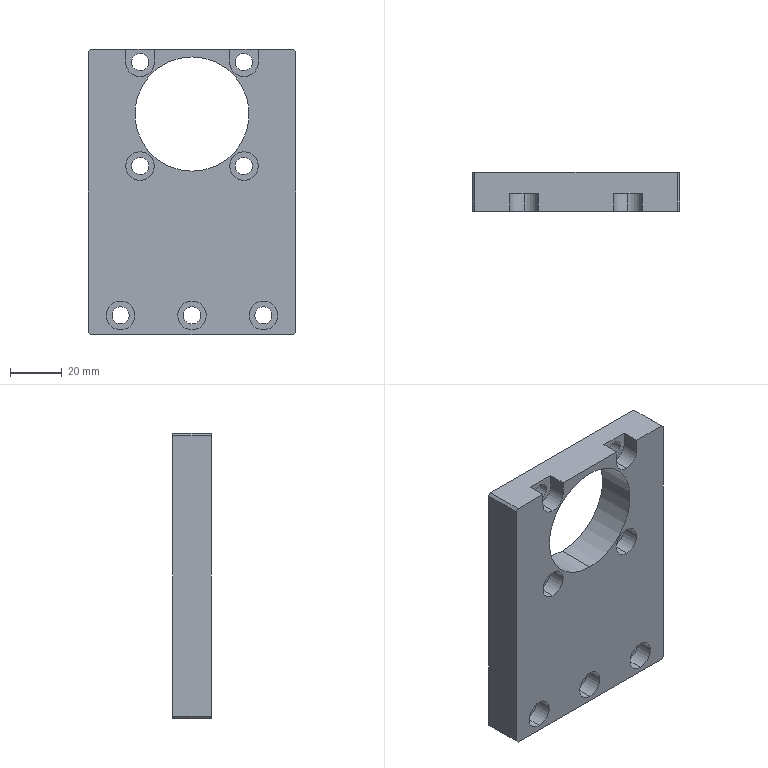Part | SolidWorks | features BaseBody 1 | 1 solid | 51 faces | box 80 x 15 x 110 mm | volume 102573 mm3 | cylinder 30 | plane 21 | commonest cylinder face diameters 6.6 x14 11 x14 44 x2
STEP:
#1=CARTESIAN_POINT('',(20.,7.5,108.3));
#2=VERTEX_POINT('',#1);
#3=CARTESIAN_POINT('',(20.,7.5,101.7));
#4=VERTEX_POINT('',#3);
#5=CARTESIAN_POINT('',(20.,7.5,105.));
#6=DIRECTION('',(0.,-1.,0.));
#7=DIRECTION('',(0.,0.,-1.));
#8=AXIS2_PLACEMENT_3D('',#5,#6,#7);
#9=CIRCLE('',#8,3.3);
#10=EDGE_CURVE('',#2,#4,#9,.T.);
#11=ORIENTED_EDGE('',*,*,#10,.F.);
#12=CARTESIAN_POINT('',(20.,-0.7,108.3));
#13=VERTEX_POINT('',#12);
#14=CARTESIAN_POINT('',(20.,-7.5,108.3));
#15=DIRECTION('',(0.,-1.,0.));
#16=VECTOR('',#15,1000.);
#17=LINE('',#14,#16);
#18=EDGE_CURVE('',#2,#13,#17,.T.);
#19=ORIENTED_EDGE('',*,*,#18,.T.);
#20=CARTESIAN_POINT('',(20.,-0.7,101.7));
#21=VERTEX_POINT('',#20);
#22=CARTESIAN_POINT('',(20.,-0.7,105.));
#23=DIRECTION('',(0.,-1.,0.));
#24=DIRECTION('',(0.,0.,-1.));
#25=AXIS2_PLACEMENT_3D('',#22,#23,#24);
#26=CIRCLE('',#25,3.3);
#27=EDGE_CURVE('',#13,#21,#26,.T.);
#28=ORIENTED_EDGE('',*,*,#27,.T.);
#29=CARTESIAN_POINT('',(20.,-7.5,101.7));
#30=DIRECTION('',(0.,-1.,0.));
#31=VECTOR('',#30,1000.);
#32=LINE('',#29,#31);
#33=EDGE_CURVE('',#4,#21,#32,.T.);
#34=ORIENTED_EDGE('',*,*,#33,.F.);
#35=EDGE_LOOP('',(#11,#19,#28,#34));
#36=FACE_OUTER_BOUND('',#35,.T.);
#37=CARTESIAN_POINT('',(20.,-7.5,105.));
#38=DIRECTION('',(0.,-1.,0.));
#39=DIRECTION('',(0.,0.,-1.));
#40=AXIS2_PLACEMENT_3D('',#37,#38,#39);
#41=CYLINDRICAL_SURFACE('',#40,3.3);
#42=ADVANCED_FACE('',(#36),#41,.F.);
#43=CARTESIAN_POINT('',(20.,-0.7,70.5));
#44=VERTEX_POINT('',#43);
#45=CARTESIAN_POINT('',(20.,-0.7,59.5));
#46=VERTEX_POINT('',#45);
#47=CARTESIAN_POINT('',(20.,-0.7,65.));
#48=DIRECTION('',(0.,-1.,0.));
#49=DIRECTION('',(0.,0.,-1.));
#50=AXIS2_PLACEMENT_3D('',#47,#48,#49);
#51=CIRCLE('',#50,5.5);
#52=EDGE_CURVE('',#44,#46,#51,.T.);
#53=ORIENTED_EDGE('',*,*,#52,.F.);
#54=CARTESIAN_POINT('',(20.,-7.5,70.5));
#55=VERTEX_POINT('',#54);
#56=CARTESIAN_POINT('',(20.,-7.5,70.5));
#57=DIRECTION('',(0.,-1.,0.));
#58=VECTOR('',#57,1000.);
#59=LINE('',#56,#58);
#60=EDGE_CURVE('',#44,#55,#59,.T.);
#61=ORIENTED_EDGE('',*,*,#60,.T.);
#62=CARTESIAN_POINT('',(20.,-7.5,59.5));
#63=VERTEX_POINT('',#62);
#64=CARTESIAN_POINT('',(20.,-7.5,65.));
#65=DIRECTION('',(0.,-1.,0.));
#66=DIRECTION('',(0.,0.,-1.));
#67=AXIS2_PLACEMENT_3D('',#64,#65,#66);
#68=CIRCLE('',#67,5.5);
#69=EDGE_CURVE('',#55,#63,#68,.T.);
#70=ORIENTED_EDGE('',*,*,#69,.T.);
#71=CARTESIAN_POINT('',(20.,-7.5,59.5));
#72=DIRECTION('',(0.,-1.,0.));
#73=VECTOR('',#72,1000.);
#74=LINE('',#71,#73);
#75=EDGE_CURVE('',#46,#63,#74,.T.);
#76=ORIENTED_EDGE('',*,*,#75,.F.);
#77=EDGE_LOOP('',(#53,#61,#70,#76));
#78=FACE_OUTER_BOUND('',#77,.T.);
#79=CARTESIAN_POINT('',(20.,-7.5,65.));
#80=DIRECTION('',(0.,-1.,0.));
#81=DIRECTION('',(0.,0.,-1.));
#82=AXIS2_PLACEMENT_3D('',#79,#80,#81);
#83=CYLINDRICAL_SURFACE('',#82,5.5);
#84=ADVANCED_FACE('',(#78),#83,.F.);
#85=CARTESIAN_POINT('',(20.,7.5,68.3));
#86=VERTEX_POINT('',#85);
#87=CARTESIAN_POINT('',(20.,7.5,61.7));
#88=VERTEX_POINT('',#87);
#89=CARTESIAN_POINT('',(20.,7.5,65.));
#90=DIRECTION('',(0.,-1.,0.));
#91=DIRECTION('',(0.,0.,-1.));
#92=AXIS2_PLACEMENT_3D('',#89,#90,#91);
#93=CIRCLE('',#92,3.3);
#94=EDGE_CURVE('',#86,#88,#93,.T.);
#95=ORIENTED_EDGE('',*,*,#94,.F.);
#96=CARTESIAN_POINT('',(20.,-0.7,68.3));
#97=VERTEX_POINT('',#96);
#98=CARTESIAN_POINT('',(20.,-7.5,68.3));
#99=DIRECTION('',(0.,-1.,0.));
#100=VECTOR('',#99,1000.);
#101=LINE('',#98,#100);
#102=EDGE_CURVE('',#86,#97,#101,.T.);
#103=ORIENTED_EDGE('',*,*,#102,.T.);
#104=CARTESIAN_POINT('',(20.,-0.7,61.7));
#105=VERTEX_POINT('',#104);
#106=CARTESIAN_POINT('',(20.,-0.7,65.));
#107=DIRECTION('',(0.,-1.,0.));
#108=DIRECTION('',(0.,0.,-1.));
#109=AXIS2_PLACEMENT_3D('',#106,#107,#108);
#110=CIRCLE('',#109,3.3);
#111=EDGE_CURVE('',#97,#105,#110,.T.);
#112=ORIENTED_EDGE('',*,*,#111,.T.);
#113=CARTESIAN_POINT('',(20.,-7.5,61.7));
#114=DIRECTION('',(0.,-1.,0.));
#115=VECTOR('',#114,1000.);
#116=LINE('',#113,#115);
#117=EDGE_CURVE('',#88,#105,#116,.T.);
#118=ORIENTED_EDGE('',*,*,#117,.F.);
#119=EDGE_LOOP('',(#95,#103,#112,#118));
#120=FACE_OUTER_BOUND('',#119,.T.);
#121=CARTESIAN_POINT('',(20.,-7.5,65.));
#122=DIRECTION('',(0.,-1.,0.));
#123=DIRECTION('',(0.,0.,-1.));
#124=AXIS2_PLACEMENT_3D('',#121,#122,#123);
#125=CYLINDRICAL_SURFACE('',#124,3.3);
#126=ADVANCED_FACE('',(#120),#125,.F.);
#127=CARTESIAN_POINT('',(-20.,-0.7,70.5));
#128=VERTEX_POINT('',#127);
#129=CARTESIAN_POINT('',(-20.,-0.7,59.5));
#130=VERTEX_POINT('',#129);
#131=CARTESIAN_POINT('',(-20.,-0.7,65.));
#132=DIRECTION('',(0.,-1.,0.));
#133=DIRECTION('',(0.,0.,-1.));
#134=AXIS2_PLACEMENT_3D('',#131,#132,#133);
#135=CIRCLE('',#134,5.5);
#136=EDGE_CURVE('',#128,#130,#135,.T.);
#137=ORIENTED_EDGE('',*,*,#136,.F.);
#138=CARTESIAN_POINT('',(-20.,-7.5,70.5));
#139=VERTEX_POINT('',#138);
#140=CARTESIAN_POINT('',(-20.,-7.5,70.5));
#141=DIRECTION('',(0.,-1.,0.));
#142=VECTOR('',#141,1000.);
#143=LINE('',#140,#142);
#144=EDGE_CURVE('',#128,#139,#143,.T.);
#145=ORIENTED_EDGE('',*,*,#144,.T.);
#146=CARTESIAN_POINT('',(-20.,-7.5,59.5));
#147=VERTEX_POINT('',#146);
#148=CARTESIAN_POINT('',(-20.,-7.5,65.));
#149=DIRECTION('',(0.,-1.,0.));
#150=DIRECTION('',(0.,0.,-1.));
#151=AXIS2_PLACEMENT_3D('',#148,#149,#150);
#152=CIRCLE('',#151,5.5);
#153=EDGE_CURVE('',#139,#147,#152,.T.);
#154=ORIENTED_EDGE('',*,*,#153,.T.);
#155=CARTESIAN_POINT('',(-20.,-7.5,59.5));
#156=DIRECTION('',(0.,-1.,0.));
#157=VECTOR('',#156,1000.);
#158=LINE('',#155,#157);
#159=EDGE_CURVE('',#130,#147,#158,.T.);
#160=ORIENTED_EDGE('',*,*,#159,.F.);
#161=EDGE_LOOP('',(#137,#145,#154,#160));
#162=FACE_OUTER_BOUND('',#161,.T.);
#163=CARTESIAN_POINT('',(-20.,-7.5,65.));
#164=DIRECTION('',(0.,-1.,0.));
#165=DIRECTION('',(0.,0.,-1.));
#166=AXIS2_PLACEMENT_3D('',#163,#164,#165);
#167=CYLINDRICAL_SURFACE('',#166,5.5);
#168=ADVANCED_FACE('',(#162),#167,.F.);
#169=CARTESIAN_POINT('',(-20.,7.5,68.3));
#170=VERTEX_POINT('',#169);
#171=CARTESIAN_POINT('',(-20.,7.5,61.7));
#172=VERTEX_POINT('',#171);
#173=CARTESIAN_POINT('',(-20.,7.5,65.));
#174=DIRECTION('',(0.,-1.,0.));
#175=DIRECTION('',(0.,0.,-1.));
#176=AXIS2_PLACEMENT_3D('',#173,#174,#175);
#177=CIRCLE('',#176,3.3);
#178=EDGE_CURVE('',#170,#172,#177,.T.);
#179=ORIENTED_EDGE('',*,*,#178,.F.);
#180=CARTESIAN_POINT('',(-20.,-0.7,68.3));
#181=VERTEX_POINT('',#180);
#182=CARTESIAN_POINT('',(-20.,-7.5,68.3));
#183=DIRECTION('',(0.,-1.,0.));
#184=VECTOR('',#183,1000.);
#185=LINE('',#182,#184);
#186=EDGE_CURVE('',#170,#181,#185,.T.);
#187=ORIENTED_EDGE('',*,*,#186,.T.);
#188=CARTESIAN_POINT('',(-20.,-0.7,61.7));
#189=VERTEX_POINT('',#188);
#190=CARTESIAN_POINT('',(-20.,-0.7,65.));
#191=DIRECTION('',(0.,-1.,0.));
#192=DIRECTION('',(0.,0.,-1.));
#193=AXIS2_PLACEMENT_3D('',#190,#191,#192);
#194=CIRCLE('',#193,3.3);
#195=EDGE_CURVE('',#181,#189,#194,.T.);
#196=ORIENTED_EDGE('',*,*,#195,.T.);
#197=CARTESIAN_POINT('',(-20.,-7.5,61.7));
#198=DIRECTION('',(0.,-1.,0.));
#199=VECTOR('',#198,1000.);
#200=LINE('',#197,#199);
#201=EDGE_CURVE('',#172,#189,#200,.T.);
#202=ORIENTED_EDGE('',*,*,#201,.F.);
#203=EDGE_LOOP('',(#179,#187,#196,#202));
#204=FACE_OUTER_BOUND('',#203,.T.);
#205=CARTESIAN_POINT('',(-20.,-7.5,65.));
#206=DIRECTION('',(0.,-1.,0.));
#207=DIRECTION('',(0.,0.,-1.));
#208=AXIS2_PLACEMENT_3D('',#205,#206,#207);
#209=CYLINDRICAL_SURFACE('',#208,3.3);
#210=ADVANCED_FACE('',(#204),#209,.F.);
#211=CARTESIAN_POINT('',(-20.,7.5,108.3));
#212=VERTEX_POINT('',#211);
#213=CARTESIAN_POINT('',(-20.,7.5,101.7));
#214=VERTEX_POINT('',#213);
#215=CARTESIAN_POINT('',(-20.,7.5,105.));
#216=DIRECTION('',(0.,-1.,0.));
#217=DIRECTION('',(0.,0.,-1.));
#218=AXIS2_PLACEMENT_3D('',#215,#216,#217);
#219=CIRCLE('',#218,3.3);
#220=EDGE_CURVE('',#212,#214,#219,.T.);
#221=ORIENTED_EDGE('',*,*,#220,.F.);
#222=CARTESIAN_POINT('',(-20.,-0.7,108.3));
#223=VERTEX_POINT('',#222);
#224=CARTESIAN_POINT('',(-20.,-7.5,108.3));
#225=DIRECTION('',(0.,-1.,0.));
#226=VECTOR('',#225,1000.);
#227=LINE('',#224,#226);
#228=EDGE_CURVE('',#212,#223,#227,.T.);
#229=ORIENTED_EDGE('',*,*,#228,.T.);
#230=CARTESIAN_POINT('',(-20.,-0.7,101.7));
#231=VERTEX_POINT('',#230);
#232=CARTESIAN_POINT('',(-20.,-0.7,105.));
#233=DIRECTION('',(0.,-1.,0.));
#234=DIRECTION('',(0.,0.,-1.));
#235=AXIS2_PLACEMENT_3D('',#232,#233,#234);
#236=CIRCLE('',#235,3.3);
#237=EDGE_CURVE('',#223,#231,#236,.T.);
#238=ORIENTED_EDGE('',*,*,#237,.T.);
#239=CARTESIAN_POINT('',(-20.,-7.5,101.7));
#240=DIRECTION('',(0.,-1.,0.));
#241=VECTOR('',#240,1000.);
#242=LINE('',#239,#241);
#243=EDGE_CURVE('',#214,#231,#242,.T.);
#244=ORIENTED_EDGE('',*,*,#243,.F.);
#245=EDGE_LOOP('',(#221,#229,#238,#244));
#246=FACE_OUTER_BOUND('',#245,.T.);
#247=CARTESIAN_POINT('',(-20.,-7.5,105.));
#248=DIRECTION('',(0.,-1.,0.));
#249=DIRECTION('',(0.,0.,-1.));
#250=AXIS2_PLACEMENT_3D('',#247,#248,#249);
#251=CYLINDRICAL_SURFACE('',#250,3.3);
#252=ADVANCED_FACE('',(#246),#251,.F.);
#253=CARTESIAN_POINT('',(27.5,-0.7,13.));
#254=VERTEX_POINT('',#253);
#255=CARTESIAN_POINT('',(27.5,-0.7,2.));
#256=VERTEX_POINT('',#255);
#257=CARTESIAN_POINT('',(27.5,-0.7,7.5));
#258=DIRECTION('',(0.,-1.,0.));
#259=DIRECTION('',(0.,0.,-1.));
#260=AXIS2_PLACEMENT_3D('',#257,#258,#259);
#261=CIRCLE('',#260,5.5);
#262=EDGE_CURVE('',#254,#256,#261,.T.);
#263=ORIENTED_EDGE('',*,*,#262,.F.);
#264=CARTESIAN_POINT('',(27.5,-7.5,13.));
#265=VERTEX_POINT('',#264);
#266=CARTESIAN_POINT('',(27.5,-7.5,13.));
#267=DIRECTION('',(0.,-1.,0.));
#268=VECTOR('',#267,1000.);
#269=LINE('',#266,#268);
#270=EDGE_CURVE('',#254,#265,#269,.T.);
#271=ORIENTED_EDGE('',*,*,#270,.T.);
#272=CARTESIAN_POINT('',(27.5,-7.5,2.));
#273=VERTEX_POINT('',#272);
#274=CARTESIAN_POINT('',(27.5,-7.5,7.5));
#275=DIRECTION('',(0.,-1.,0.));
#276=DIRECTION('',(0.,0.,-1.));
#277=AXIS2_PLACEMENT_3D('',#274,#275,#276);
#278=CIRCLE('',#277,5.5);
#279=EDGE_CURVE('',#265,#273,#278,.T.);
#280=ORIENTED_EDGE('',*,*,#279,.T.);
#281=CARTESIAN_POINT('',(27.5,-7.5,2.));
#282=DIRECTION('',(0.,-1.,0.));
#283=VECTOR('',#282,1000.);
#284=LINE('',#281,#283);
#285=EDGE_CURVE('',#256,#273,#284,.T.);
#286=ORIENTED_EDGE('',*,*,#285,.F.);
#287=EDGE_LOOP('',(#263,#271,#280,#286));
#288=FACE_OUTER_BOUND('',#287,.T.);
#289=CARTESIAN_POINT('',(27.5,-7.5,7.5));
#290=DIRECTION('',(0.,-1.,0.));
#291=DIRECTION('',(0.,0.,-1.));
#292=AXIS2_PLACEMENT_3D('',#289,#290,#291);
#293=CYLINDRICAL_SURFACE('',#292,5.5);
#294=ADVANCED_FACE('',(#288),#293,.F.);
#295=CARTESIAN_POINT('',(27.5,7.5,10.8));
#296=VERTEX_POINT('',#295);
#297=CARTESIAN_POINT('',(27.5,7.5,4.2));
#298=VERTEX_POINT('',#297);
#299=CARTESIAN_POINT('',(27.5,7.5,7.5));
#300=DIRECTION('',(0.,-1.,0.));
#301=DIRECTION('',(0.,0.,-1.));
#302=AXIS2_PLACEMENT_3D('',#299,#300,#301);
#303=CIRCLE('',#302,3.3);
#304=EDGE_CURVE('',#296,#298,#303,.T.);
#305=ORIENTED_EDGE('',*,*,#304,.F.);
#306=CARTESIAN_POINT('',(27.5,-0.7,10.8));
#307=VERTEX_POINT('',#306);
#308=CARTESIAN_POINT('',(27.5,-7.5,10.8));
#309=DIRECTION('',(0.,-1.,0.));
#310=VECTOR('',#309,1000.);
#311=LINE('',#308,#310);
#312=EDGE_CURVE('',#296,#307,#311,.T.);
#313=ORIENTED_EDGE('',*,*,#312,.T.);
#314=CARTESIAN_POINT('',(27.5,-0.7,4.2));
#315=VERTEX_POINT('',#314);
#316=CARTESIAN_POINT('',(27.5,-0.7,7.5));
#317=DIRECTION('',(0.,-1.,0.));
#318=DIRECTION('',(0.,0.,-1.));
#319=AXIS2_PLACEMENT_3D('',#316,#317,#318);
#320=CIRCLE('',#319,3.3);
#321=EDGE_CURVE('',#307,#315,#320,.T.);
#322=ORIENTED_EDGE('',*,*,#321,.T.);
#323=CARTESIAN_POINT('',(27.5,-7.5,4.2));
#324=DIRECTION('',(0.,-1.,0.));
#325=VECTOR('',#324,1000.);
#326=LINE('',#323,#325);
#327=EDGE_CURVE('',#298,#315,#326,.T.);
#328=ORIENTED_EDGE('',*,*,#327,.F.);
#329=EDGE_LOOP('',(#305,#313,#322,#328));
#330=FACE_OUTER_BOUND('',#329,.T.);
#331=CARTESIAN_POINT('',(27.5,-7.5,7.5));
#332=DIRECTION('',(0.,-1.,0.));
#333=DIRECTION('',(0.,0.,-1.));
#334=AXIS2_PLACEMENT_3D('',#331,#332,#333);
#335=CYLINDRICAL_SURFACE('',#334,3.3);
#336=ADVANCED_FACE('',(#330),#335,.F.);
#337=CARTESIAN_POINT('',(-27.5,-0.7,13.));
#338=VERTEX_POINT('',#337);
#339=CARTESIAN_POINT('',(-27.5,-0.7,2.));
#340=VERTEX_POINT('',#339);
#341=CARTESIAN_POINT('',(-27.5,-0.7,7.5));
#342=DIRECTION('',(0.,-1.,0.));
#343=DIRECTION('',(0.,0.,-1.));
#344=AXIS2_PLACEMENT_3D('',#341,#342,#343);
#345=CIRCLE('',#344,5.5);
#346=EDGE_CURVE('',#338,#340,#345,.T.);
#347=ORIENTED_EDGE('',*,*,#346,.F.);
#348=CARTESIAN_POINT('',(-27.5,-7.5,13.));
#349=VERTEX_POINT('',#348);
#350=CARTESIAN_POINT('',(-27.5,-7.5,13.));
#351=DIRECTION('',(0.,-1.,0.));
#352=VECTOR('',#351,1000.);
#353=LINE('',#350,#352);
#354=EDGE_CURVE('',#338,#349,#353,.T.);
#355=ORIENTED_EDGE('',*,*,#354,.T.);
#356=CARTESIAN_POINT('',(-27.5,-7.5,2.));
#357=VERTEX_POINT('',#356);
#358=CARTESIAN_POINT('',(-27.5,-7.5,7.5));
#359=DIRECTION('',(0.,-1.,0.));
#360=DIRECTION('',(0.,0.,-1.));
#361=AXIS2_PLACEMENT_3D('',#358,#359,#360);
#362=CIRCLE('',#361,5.5);
#363=EDGE_CURVE('',#349,#357,#362,.T.);
#364=ORIENTED_EDGE('',*,*,#363,.T.);
#365=CARTESIAN_POINT('',(-27.5,-7.5,2.));
#366=DIRECTION('',(0.,-1.,0.));
#367=VECTOR('',#366,1000.);
#368=LINE('',#365,#367);
#369=EDGE_CURVE('',#340,#357,#368,.T.);
#370=ORIENTED_EDGE('',*,*,#369,.F.);
#371=EDGE_LOOP('',(#347,#355,#364,#370));
#372=FACE_OUTER_BOUND('',#371,.T.);
#373=CARTESIAN_POINT('',(-27.5,-7.5,7.5));
#374=DIRECTION('',(0.,-1.,0.));
#375=DIRECTION('',(0.,0.,-1.));
#376=AXIS2_PLACEMENT_3D('',#373,#374,#375);
#377=CYLINDRICAL_SURFACE('',#376,5.5);
#378=ADVANCED_FACE('',(#372),#377,.F.);
#379=CARTESIAN_POINT('',(-27.5,7.5,10.8));
#380=VERTEX_POINT('',#379);
#381=CARTESIAN_POINT('',(-27.5,7.5,4.2));
#382=VERTEX_POINT('',#381);
#383=CARTESIAN_POINT('',(-27.5,7.5,7.5));
#384=DIRECTION('',(0.,-1.,0.));
#385=DIRECTION('',(0.,0.,-1.));
#386=AXIS2_PLACEMENT_3D('',#383,#384,#385);
#387=CIRCLE('',#386,3.3);
#388=EDGE_CURVE('',#380,#382,#387,.T.);
#389=ORIENTED_EDGE('',*,*,#388,.F.);
#390=CARTESIAN_POINT('',(-27.5,-0.7,10.8));
#391=VERTEX_POINT('',#390);
#392=CARTESIAN_POINT('',(-27.5,-7.5,10.8));
#393=DIRECTION('',(0.,-1.,0.));
#394=VECTOR('',#393,1000.);
#395=LINE('',#392,#394);
#396=EDGE_CURVE('',#380,#391,#395,.T.);
#397=ORIENTED_EDGE('',*,*,#396,.T.);
#398=CARTESIAN_POINT('',(-27.5,-0.7,4.2));
#399=VERTEX_POINT('',#398);
#400=CARTESIAN_POINT('',(-27.5,-0.7,7.5));
#401=DIRECTION('',(0.,-1.,0.));
#402=DIRECTION('',(0.,0.,-1.));
#403=AXIS2_PLACEMENT_3D('',#400,#401,#402);
#404=CIRCLE('',#403,3.3);
#405=EDGE_CURVE('',#391,#399,#404,.T.);
#406=ORIENTED_EDGE('',*,*,#405,.T.);
#407=CARTESIAN_POINT('',(-27.5,-7.5,4.2));
#408=DIRECTION('',(0.,-1.,0.));
#409=VECTOR('',#408,1000.);
#410=LINE('',#407,#409);
#411=EDGE_CURVE('',#382,#399,#410,.T.);
#412=ORIENTED_EDGE('',*,*,#411,.F.);
#413=EDGE_LOOP('',(#389,#397,#406,#412));
#414=FACE_OUTER_BOUND('',#413,.T.);
#415=CARTESIAN_POINT('',(-27.5,-7.5,7.5));
#416=DIRECTION('',(0.,-1.,0.));
#417=DIRECTION('',(0.,0.,-1.));
#418=AXIS2_PLACEMENT_3D('',#415,#416,#417);
#419=CYLINDRICAL_SURFACE('',#418,3.3);
#420=ADVANCED_FACE('',(#414),#419,.F.);
#421=CARTESIAN_POINT('',(0.,-0.7,13.));
#422=VERTEX_POINT('',#421);
#423=CARTESIAN_POINT('',(0.,-0.7,2.));
#424=VERTEX_POINT('',#423);
#425=CARTESIAN_POINT('',(0.,-0.7,7.5));
#426=DIRECTION('',(0.,-1.,0.));
#427=DIRECTION('',(0.,0.,-1.));
#428=AXIS2_PLACEMENT_3D('',#425,#426,#427);
#429=CIRCLE('',#428,5.5);
#430=EDGE_CURVE('',#422,#424,#429,.T.);
#431=ORIENTED_EDGE('',*,*,#430,.F.);
#432=CARTESIAN_POINT('',(0.,-7.5,13.));
#433=VERTEX_POINT('',#432);
#434=CARTESIAN_POINT('',(0.,-7.5,13.));
#435=DIRECTION('',(0.,-1.,0.));
#436=VECTOR('',#435,1000.);
#437=LINE('',#434,#436);
#438=EDGE_CURVE('',#422,#433,#437,.T.);
#439=ORIENTED_EDGE('',*,*,#438,.T.);
#440=CARTESIAN_POINT('',(0.,-7.5,2.));
#441=VERTEX_POINT('',#440);
#442=CARTESIAN_POINT('',(0.,-7.5,7.5));
#443=DIRECTION('',(0.,-1.,0.));
#444=DIRECTION('',(0.,0.,-1.));
#445=AXIS2_PLACEMENT_3D('',#442,#443,#444);
#446=CIRCLE('',#445,5.5);
#447=EDGE_CURVE('',#433,#441,#446,.T.);
#448=ORIENTED_EDGE('',*,*,#447,.T.);
#449=CARTESIAN_POINT('',(0.,-7.5,2.));
#450=DIRECTION('',(0.,-1.,0.));
#451=VECTOR('',#450,1000.);
#452=LINE('',#449,#451);
#453=EDGE_CURVE('',#424,#441,#452,.T.);
#454=ORIENTED_EDGE('',*,*,#453,.F.);
#455=EDGE_LOOP('',(#431,#439,#448,#454));
#456=FACE_OUTER_BOUND('',#455,.T.);
#457=CARTESIAN_POINT('',(0.,-7.5,7.5));
#458=DIRECTION('',(0.,-1.,0.));
#459=DIRECTION('',(0.,0.,-1.));
#460=AXIS2_PLACEMENT_3D('',#457,#458,#459);
#461=CYLINDRICAL_SURFACE('',#460,5.5);
#462=ADVANCED_FACE('',(#456),#461,.F.);
#463=CARTESIAN_POINT('',(0.,7.5,10.8));
#464=VERTEX_POINT('',#463);
#465=CARTESIAN_POINT('',(0.,7.5,4.2));
#466=VERTEX_POINT('',#465);
#467=CARTESIAN_POINT('',(0.,7.5,7.5));
#468=DIRECTION('',(0.,-1.,0.));
#469=DIRECTION('',(0.,0.,-1.));
#470=AXIS2_PLACEMENT_3D('',#467,#468,#469);
#471=CIRCLE('',#470,3.3);
#472=EDGE_CURVE('',#464,#466,#471,.T.);
#473=ORIENTED_EDGE('',*,*,#472,.F.);
#474=CARTESIAN_POINT('',(0.,-0.7,10.8));
#475=VERTEX_POINT('',#474);
#476=CARTESIAN_POINT('',(0.,-7.5,10.8));
#477=DIRECTION('',(0.,-1.,0.));
#478=VECTOR('',#477,1000.);
#479=LINE('',#476,#478);
#480=EDGE_CURVE('',#464,#475,#479,.T.);
#481=ORIENTED_EDGE('',*,*,#480,.T.);
#482=CARTESIAN_POINT('',(0.,-0.7,4.2));
#483=VERTEX_POINT('',#482);
#484=CARTESIAN_POINT('',(0.,-0.7,7.5));
#485=DIRECTION('',(0.,-1.,0.));
#486=DIRECTION('',(0.,0.,-1.));
#487=AXIS2_PLACEMENT_3D('',#484,#485,#486);
#488=CIRCLE('',#487,3.3);
#489=EDGE_CURVE('',#475,#483,#488,.T.);
#490=ORIENTED_EDGE('',*,*,#489,.T.);
#491=CARTESIAN_POINT('',(0.,-7.5,4.2));
#492=DIRECTION('',(0.,-1.,0.));
#493=VECTOR('',#492,1000.);
#494=LINE('',#491,#493);
#495=EDGE_CURVE('',#466,#483,#494,.T.);
#496=ORIENTED_EDGE('',*,*,#495,.F.);
#497=EDGE_LOOP('',(#473,#481,#490,#496));
#498=FACE_OUTER_BOUND('',#497,.T.);
#499=CARTESIAN_POINT('',(0.,-7.5,7.5));
#500=DIRECTION('',(0.,-1.,0.));
#501=DIRECTION('',(0.,0.,-1.));
#502=AXIS2_PLACEMENT_3D('',#499,#500,#501);
#503=CYLINDRICAL_SURFACE('',#502,3.3);
#504=ADVANCED_FACE('',(#498),#503,.F.);
#505=CARTESIAN_POINT('',(0.,7.5,107.));
#506=VERTEX_POINT('',#505);
#507=CARTESIAN_POINT('',(0.,7.5,63.));
#508=VERTEX_POINT('',#507);
#509=CARTESIAN_POINT('',(0.,7.5,85.));
#510=DIRECTION('',(0.,-1.,0.));
#511=DIRECTION('',(0.,0.,-1.));
#512=AXIS2_PLACEMENT_3D('',#509,#510,#511);
#513=CIRCLE('',#512,22.);
#514=EDGE_CURVE('',#506,#508,#513,.T.);
#515=ORIENTED_EDGE('',*,*,#514,.F.);
#516=CARTESIAN_POINT('',(0.,-7.5,107.));
#517=VERTEX_POINT('',#516);
#518=CARTESIAN_POINT('',(0.,7.5,107.));
#519=DIRECTION('',(0.,-1.,0.));
#520=VECTOR('',#519,1000.);
#521=LINE('',#518,#520);
#522=EDGE_CURVE('',#506,#517,#521,.T.);
#523=ORIENTED_EDGE('',*,*,#522,.T.);
#524=CARTESIAN_POINT('',(0.,-7.5,63.));
#525=VERTEX_POINT('',#524);
#526=CARTESIAN_POINT('',(0.,-7.5,85.));
#527=DIRECTION('',(0.,-1.,0.));
#528=DIRECTION('',(0.,0.,-1.));
#529=AXIS2_PLACEMENT_3D('',#526,#527,#528);
#530=CIRCLE('',#529,22.);
#531=EDGE_CURVE('',#517,#525,#530,.T.);
#532=ORIENTED_EDGE('',*,*,#531,.T.);
#533=CARTESIAN_POINT('',(0.,7.5,63.));
#534=DIRECTION('',(0.,-1.,0.));
#535=VECTOR('',#534,1000.);
#536=LINE('',#533,#535);
#537=EDGE_CURVE('',#508,#525,#536,.T.);
#538=ORIENTED_EDGE('',*,*,#537,.F.);
#539=EDGE_LOOP('',(#515,#523,#532,#538));
#540=FACE_OUTER_BOUND('',#539,.T.);
#541=CARTESIAN_POINT('',(0.,7.5,85.));
#542=DIRECTION('',(0.,-1.,0.));
#543=DIRECTION('',(0.,0.,-1.));
#544=AXIS2_PLACEMENT_3D('',#541,#542,#543);
#545=CYLINDRICAL_SURFACE('',#544,22.);
#546=ADVANCED_FACE('',(#540),#545,.F.);
#547=CARTESIAN_POINT('',(20.,-0.7,99.5));
#548=VERTEX_POINT('',#547);
#549=CARTESIAN_POINT('',(25.5,-0.7,105.));
#550=VERTEX_POINT('',#549);
#551=CARTESIAN_POINT('',(20.,-0.7,105.));
#552=DIRECTION('',(0.,-1.,0.));
#553=DIRECTION('',(0.,0.,-1.));
#554=AXIS2_PLACEMENT_3D('',#551,#552,#553);
#555=CIRCLE('',#554,5.5);
#556=EDGE_CURVE('',#548,#550,#555,.T.);
#557=ORIENTED_EDGE('',*,*,#556,.F.);
#558=CARTESIAN_POINT('',(20.,-7.5,99.5));
#559=VERTEX_POINT('',#558);
#560=CARTESIAN_POINT('',(20.,-7.5,99.5));
#561=DIRECTION('',(0.,-1.,0.));
#562=VECTOR('',#561,1000.);
#563=LINE('',#560,#562);
#564=EDGE_CURVE('',#548,#559,#563,.T.);
#565=ORIENTED_EDGE('',*,*,#564,.T.);
#566=CARTESIAN_POINT('',(25.5,-7.5,105.));
#567=VERTEX_POINT('',#566);
#568=CARTESIAN_POINT('',(20.,-7.5,105.));
#569=DIRECTION('',(0.,-1.,0.));
#570=DIRECTION('',(0.,0.,-1.));
#571=AXIS2_PLACEMENT_3D('',#568,#569,#570);
#572=CIRCLE('',#571,5.5);
#573=EDGE_CURVE('',#559,#567,#572,.T.);
#574=ORIENTED_EDGE('',*,*,#573,.T.);
#575=CARTESIAN_POINT('',(25.5,11.383,105.));
#576=DIRECTION('',(0.,-1.,0.));
#577=VECTOR('',#576,1000.);
#578=LINE('',#575,#577);
#579=EDGE_CURVE('',#550,#567,#578,.T.);
#580=ORIENTED_EDGE('',*,*,#579,.F.);
#581=EDGE_LOOP('',(#557,#565,#574,#580));
#582=FACE_OUTER_BOUND('',#581,.T.);
#583=CARTESIAN_POINT('',(20.,-7.5,105.));
#584=DIRECTION('',(0.,-1.,0.));
#585=DIRECTION('',(0.,0.,-1.));
#586=AXIS2_PLACEMENT_3D('',#583,#584,#585);
#587=CYLINDRICAL_SURFACE('',#586,5.5);
#588=ADVANCED_FACE('',(#582),#587,.F.);
#589=CARTESIAN_POINT('',(-20.,-0.7,99.5));
#590=VERTEX_POINT('',#589);
#591=CARTESIAN_POINT('',(-14.5,-0.7,105.));
#592=VERTEX_POINT('',#591);
#593=CARTESIAN_POINT('',(-20.,-0.7,105.));
#594=DIRECTION('',(0.,-1.,0.));
#595=DIRECTION('',(0.,0.,-1.));
#596=AXIS2_PLACEMENT_3D('',#593,#594,#595);
#597=CIRCLE('',#596,5.5);
#598=EDGE_CURVE('',#590,#592,#597,.T.);
#599=ORIENTED_EDGE('',*,*,#598,.F.);
#600=CARTESIAN_POINT('',(-20.,-7.5,99.5));
#601=VERTEX_POINT('',#600);
#602=CARTESIAN_POINT('',(-20.,-7.5,99.5));
#603=DIRECTION('',(0.,-1.,0.));
#604=VECTOR('',#603,1000.);
#605=LINE('',#602,#604);
#606=EDGE_CURVE('',#590,#601,#605,.T.);
#607=ORIENTED_EDGE('',*,*,#606,.T.);
#608=CARTESIAN_POINT('',(-14.5,-7.5,105.));
#609=VERTEX_POINT('',#608);
#610=CARTESIAN_POINT('',(-20.,-7.5,105.));
#611=DIRECTION('',(0.,-1.,0.));
#612=DIRECTION('',(0.,0.,-1.));
#613=AXIS2_PLACEMENT_3D('',#610,#611,#612);
#614=CIRCLE('',#613,5.5);
#615=EDGE_CURVE('',#601,#609,#614,.T.);
#616=ORIENTED_EDGE('',*,*,#615,.T.);
#617=CARTESIAN_POINT('',(-14.5,11.383,105.));
#618=DIRECTION('',(0.,-1.,0.));
#619=VECTOR('',#618,1000.);
#620=LINE('',#617,#619);
#621=EDGE_CURVE('',#592,#609,#620,.T.);
#622=ORIENTED_EDGE('',*,*,#621,.F.);
#623=EDGE_LOOP('',(#599,#607,#616,#622));
#624=FACE_OUTER_BOUND('',#623,.T.);
#625=CARTESIAN_POINT('',(-20.,-7.5,105.));
#626=DIRECTION('',(0.,-1.,0.));
#627=DIRECTION('',(0.,0.,-1.));
#628=AXIS2_PLACEMENT_3D('',#625,#626,#627);
#629=CYLINDRICAL_SURFACE('',#628,5.5);
#630=ADVANCED_FACE('',(#624),#629,.F.);
#631=CARTESIAN_POINT('',(39.,-7.5,0.));
#632=VERTEX_POINT('',#631);
#633=CARTESIAN_POINT('',(40.,-7.5,1.));
#634=VERTEX_POINT('',#633);
#635=CARTESIAN_POINT('',(40.,-7.5,1.));
#636=DIRECTION('',(0.7071,0.,0.7071));
#637=VECTOR('',#636,1000.);
#638=LINE('',#635,#637);
#639=EDGE_CURVE('',#632,#634,#638,.T.);
#640=ORIENTED_EDGE('',*,*,#639,.F.);
#641=CARTESIAN_POINT('',(39.,7.5,0.));
#642=VERTEX_POINT('',#641);
#643=CARTESIAN_POINT('',(39.,-7.5,0.));
#644=DIRECTION('',(0.,-1.,0.));
#645=VECTOR('',#644,1000.);
#646=LINE('',#643,#645);
#647=EDGE_CURVE('',#642,#632,#646,.T.);
#648=ORIENTED_EDGE('',*,*,#647,.F.);
#649=CARTESIAN_POINT('',(40.,7.5,1.));
#650=VERTEX_POINT('',#649);
#651=CARTESIAN_POINT('',(40.,7.5,1.));
#652=DIRECTION('',(-0.7071,0.,-0.7071));
#653=VECTOR('',#652,1000.);
#654=LINE('',#651,#653);
#655=EDGE_CURVE('',#650,#642,#654,.T.);
#656=ORIENTED_EDGE('',*,*,#655,.F.);
#657=CARTESIAN_POINT('',(40.,7.5,1.));
#658=DIRECTION('',(0.,1.,0.));
#659=VECTOR('',#658,1000.);
#660=LINE('',#657,#659);
#661=EDGE_CURVE('',#634,#650,#660,.T.);
#662=ORIENTED_EDGE('',*,*,#661,.F.);
#663=EDGE_LOOP('',(#640,#648,#656,#662));
#664=FACE_OUTER_BOUND('',#663,.T.);
#665=CARTESIAN_POINT('',(40.,-7.5,1.));
#666=DIRECTION('',(0.7071,0.,-0.7071));
#667=DIRECTION('',(0.,-1.,0.));
#668=AXIS2_PLACEMENT_3D('',#665,#666,#667);
#669=PLANE('',#668);
#670=ADVANCED_FACE('',(#664),#669,.T.);
#671=CARTESIAN_POINT('',(40.,-7.5,109.));
#672=VERTEX_POINT('',#671);
#673=CARTESIAN_POINT('',(39.,-7.5,110.));
#674=VERTEX_POINT('',#673);
#675=CARTESIAN_POINT('',(39.,-7.5,110.));
#676=DIRECTION('',(-0.7071,0.,0.7071));
#677=VECTOR('',#676,1000.);
#678=LINE('',#675,#677);
#679=EDGE_CURVE('',#672,#674,#678,.T.);
#680=ORIENTED_EDGE('',*,*,#679,.F.);
#681=CARTESIAN_POINT('',(40.,7.5,109.));
#682=VERTEX_POINT('',#681);
#683=CARTESIAN_POINT('',(40.,-7.5,109.));
#684=DIRECTION('',(0.,-1.,0.));
#685=VECTOR('',#684,1000.);
#686=LINE('',#683,#685);
#687=EDGE_CURVE('',#682,#672,#686,.T.);
#688=ORIENTED_EDGE('',*,*,#687,.F.);
#689=CARTESIAN_POINT('',(39.,7.5,110.));
#690=VERTEX_POINT('',#689);
#691=CARTESIAN_POINT('',(39.,7.5,110.));
#692=DIRECTION('',(0.7071,0.,-0.7071));
#693=VECTOR('',#692,1000.);
#694=LINE('',#691,#693);
#695=EDGE_CURVE('',#690,#682,#694,.T.);
#696=ORIENTED_EDGE('',*,*,#695,.F.);
#697=CARTESIAN_POINT('',(39.,0.,110.));
#698=DIRECTION('',(0.,1.,0.));
#699=VECTOR('',#698,1000.);
#700=LINE('',#697,#699);
#701=EDGE_CURVE('',#674,#690,#700,.T.);
#702=ORIENTED_EDGE('',*,*,#701,.F.);
#703=EDGE_LOOP('',(#680,#688,#696,#702));
#704=FACE_OUTER_BOUND('',#703,.T.);
#705=CARTESIAN_POINT('',(39.,0.,110.));
#706=DIRECTION('',(-0.7071,0.,-0.7071));
#707=DIRECTION('',(-0.7071,0.,0.7071));
#708=AXIS2_PLACEMENT_3D('',#705,#706,#707);
#709=PLANE('',#708);
#710=ADVANCED_FACE('',(#704),#709,.F.);
#711=CARTESIAN_POINT('',(-39.,7.5,0.));
#712=VERTEX_POINT('',#711);
#713=CARTESIAN_POINT('',(-40.,7.5,1.));
#714=VERTEX_POINT('',#713);
#715=CARTESIAN_POINT('',(-40.,7.5,1.));
#716=DIRECTION('',(-0.7071,0.,0.7071));
#717=VECTOR('',#716,1000.);
#718=LINE('',#715,#717);
#719=EDGE_CURVE('',#712,#714,#718,.T.);
#720=ORIENTED_EDGE('',*,*,#719,.F.);
#721=CARTESIAN_POINT('',(-39.,-7.5,0.));
#722=VERTEX_POINT('',#721);
#723=CARTESIAN_POINT('',(-39.,7.5,0.));
#724=DIRECTION('',(0.,1.,0.));
#725=VECTOR('',#724,1000.);
#726=LINE('',#723,#725);
#727=EDGE_CURVE('',#722,#712,#726,.T.);
#728=ORIENTED_EDGE('',*,*,#727,.F.);
#729=CARTESIAN_POINT('',(-40.,-7.5,1.));
#730=VERTEX_POINT('',#729);
#731=CARTESIAN_POINT('',(-40.,-7.5,1.));
#732=DIRECTION('',(0.7071,0.,-0.7071));
#733=VECTOR('',#732,1000.);
#734=LINE('',#731,#733);
#735=EDGE_CURVE('',#730,#722,#734,.T.);
#736=ORIENTED_EDGE('',*,*,#735,.F.);
#737=CARTESIAN_POINT('',(-40.,-7.5,1.));
#738=DIRECTION('',(0.,-1.,0.));
#739=VECTOR('',#738,1000.);
#740=LINE('',#737,#739);
#741=EDGE_CURVE('',#714,#730,#740,.T.);
#742=ORIENTED_EDGE('',*,*,#741,.F.);
#743=EDGE_LOOP('',(#720,#728,#736,#742));
#744=FACE_OUTER_BOUND('',#743,.T.);
#745=CARTESIAN_POINT('',(-40.,-7.5,1.));
#746=DIRECTION('',(-0.7071,0.,-0.7071));
#747=DIRECTION('',(-0.7071,0.,0.7071));
#748=AXIS2_PLACEMENT_3D('',#745,#746,#747);
#749=PLANE('',#748);
#750=ADVANCED_FACE('',(#744),#749,.T.);
#751=CARTESIAN_POINT('',(-40.,7.5,109.));
#752=VERTEX_POINT('',#751);
#753=CARTESIAN_POINT('',(-39.,7.5,110.));
#754=VERTEX_POINT('',#753);
#755=CARTESIAN_POINT('',(-39.,7.5,110.));
#756=DIRECTION('',(0.7071,0.,0.7071));
#757=VECTOR('',#756,1000.);
#758=LINE('',#755,#757);
#759=EDGE_CURVE('',#752,#754,#758,.T.);
#760=ORIENTED_EDGE('',*,*,#759,.F.);
#761=CARTESIAN_POINT('',(-40.,-7.5,109.));
#762=VERTEX_POINT('',#761);
#763=CARTESIAN_POINT('',(-40.,-7.5,109.));
#764=DIRECTION('',(0.,1.,0.));
#765=VECTOR('',#764,1000.);
#766=LINE('',#763,#765);
#767=EDGE_CURVE('',#762,#752,#766,.T.);
#768=ORIENTED_EDGE('',*,*,#767,.F.);
#769=CARTESIAN_POINT('',(-39.,-7.5,110.));
#770=VERTEX_POINT('',#769);
#771=CARTESIAN_POINT('',(-39.,-7.5,110.));
#772=DIRECTION('',(-0.7071,0.,-0.7071));
#773=VECTOR('',#772,1000.);
#774=LINE('',#771,#773);
#775=EDGE_CURVE('',#770,#762,#774,.T.);
#776=ORIENTED_EDGE('',*,*,#775,.F.);
#777=CARTESIAN_POINT('',(-39.,0.,110.));
#778=DIRECTION('',(0.,-1.,0.));
#779=VECTOR('',#778,1000.);
#780=LINE('',#777,#779);
#781=EDGE_CURVE('',#754,#770,#780,.T.);
#782=ORIENTED_EDGE('',*,*,#781,.F.);
#783=EDGE_LOOP('',(#760,#768,#776,#782));
#784=FACE_OUTER_BOUND('',#783,.T.);
#785=CARTESIAN_POINT('',(-39.,0.,110.));
#786=DIRECTION('',(0.7071,0.,-0.7071));
#787=DIRECTION('',(0.,-1.,0.));
#788=AXIS2_PLACEMENT_3D('',#785,#786,#787);
#789=PLANE('',#788);
#790=ADVANCED_FACE('',(#784),#789,.F.);
#791=ORIENTED_EDGE('',*,*,#621,.T.);
#792=CARTESIAN_POINT('',(-14.5,-7.5,110.));
#793=VERTEX_POINT('',#792);
#794=CARTESIAN_POINT('',(-14.5,-7.5,105.));
#795=DIRECTION('',(0.,0.,1.));
#796=VECTOR('',#795,1000.);
#797=LINE('',#794,#796);
#798=EDGE_CURVE('',#609,#793,#797,.T.);
#799=ORIENTED_EDGE('',*,*,#798,.T.);
#800=CARTESIAN_POINT('',(-14.5,-0.7,110.));
#801=VERTEX_POINT('',#800);
#802=CARTESIAN_POINT('',(-14.5,11.383,110.));
#803=DIRECTION('',(0.,-1.,0.));
#804=VECTOR('',#803,1000.);
#805=LINE('',#802,#804);
#806=EDGE_CURVE('',#801,#793,#805,.T.);
#807=ORIENTED_EDGE('',*,*,#806,.F.);
#808=CARTESIAN_POINT('',(-14.5,-0.7,105.));
#809=DIRECTION('',(0.,0.,1.));
#810=VECTOR('',#809,1000.);
#811=LINE('',#808,#810);
#812=EDGE_CURVE('',#592,#801,#811,.T.);
#813=ORIENTED_EDGE('',*,*,#812,.F.);
#814=EDGE_LOOP('',(#791,#799,#807,#813));
#815=FACE_OUTER_BOUND('',#814,.T.);
#816=CARTESIAN_POINT('',(-14.5,11.383,105.));
#817=DIRECTION('',(1.,0.,0.));
#818=DIRECTION('',(0.,1.,0.));
#819=AXIS2_PLACEMENT_3D('',#816,#817,#818);
#820=PLANE('',#819);
#821=ADVANCED_FACE('',(#815),#820,.F.);
#822=CARTESIAN_POINT('',(-25.5,-0.7,110.));
#823=VERTEX_POINT('',#822);
#824=CARTESIAN_POINT('',(-25.5,-7.5,110.));
#825=VERTEX_POINT('',#824);
#826=CARTESIAN_POINT('',(-25.5,11.383,110.));
#827=DIRECTION('',(0.,-1.,0.));
#828=VECTOR('',#827,1000.);
#829=LINE('',#826,#828);
#830=EDGE_CURVE('',#823,#825,#829,.T.);
#831=ORIENTED_EDGE('',*,*,#830,.T.);
#832=CARTESIAN_POINT('',(-25.5,-7.5,105.));
#833=VERTEX_POINT('',#832);
#834=CARTESIAN_POINT('',(-25.5,-7.5,105.));
#835=DIRECTION('',(0.,0.,-1.));
#836=VECTOR('',#835,1000.);
#837=LINE('',#834,#836);
#838=EDGE_CURVE('',#825,#833,#837,.T.);
#839=ORIENTED_EDGE('',*,*,#838,.T.);
#840=CARTESIAN_POINT('',(-25.5,-0.7,105.));
#841=VERTEX_POINT('',#840);
#842=CARTESIAN_POINT('',(-25.5,11.383,105.));
#843=DIRECTION('',(0.,-1.,0.));
#844=VECTOR('',#843,1000.);
#845=LINE('',#842,#844);
#846=EDGE_CURVE('',#841,#833,#845,.T.);
#847=ORIENTED_EDGE('',*,*,#846,.F.);
#848=CARTESIAN_POINT('',(-25.5,-0.7,105.));
#849=DIRECTION('',(0.,0.,-1.));
#850=VECTOR('',#849,1000.);
#851=LINE('',#848,#850);
#852=EDGE_CURVE('',#823,#841,#851,.T.);
#853=ORIENTED_EDGE('',*,*,#852,.F.);
#854=EDGE_LOOP('',(#831,#839,#847,#853));
#855=FACE_OUTER_BOUND('',#854,.T.);
#856=CARTESIAN_POINT('',(-25.5,11.383,105.));
#857=DIRECTION('',(-1.,0.,0.));
#858=DIRECTION('',(0.,0.,1.));
#859=AXIS2_PLACEMENT_3D('',#856,#857,#858);
#860=PLANE('',#859);
#861=ADVANCED_FACE('',(#855),#860,.F.);
#862=ORIENTED_EDGE('',*,*,#579,.T.);
#863=CARTESIAN_POINT('',(25.5,-7.5,110.));
#864=VERTEX_POINT('',#863);
#865=CARTESIAN_POINT('',(25.5,-7.5,105.));
#866=DIRECTION('',(0.,0.,1.));
#867=VECTOR('',#866,1000.);
#868=LINE('',#865,#867);
#869=EDGE_CURVE('',#567,#864,#868,.T.);
#870=ORIENTED_EDGE('',*,*,#869,.T.);
#871=CARTESIAN_POINT('',(25.5,-0.7,110.));
#872=VERTEX_POINT('',#871);
#873=CARTESIAN_POINT('',(25.5,11.383,110.));
#874=DIRECTION('',(0.,-1.,0.));
#875=VECTOR('',#874,1000.);
#876=LINE('',#873,#875);
#877=EDGE_CURVE('',#872,#864,#876,.T.);
#878=ORIENTED_EDGE('',*,*,#877,.F.);
#879=CARTESIAN_POINT('',(25.5,-0.7,105.));
#880=DIRECTION('',(0.,0.,1.));
#881=VECTOR('',#880,1000.);
#882=LINE('',#879,#881);
#883=EDGE_CURVE('',#550,#872,#882,.T.);
#884=ORIENTED_EDGE('',*,*,#883,.F.);
#885=EDGE_LOOP('',(#862,#870,#878,#884));
#886=FACE_OUTER_BOUND('',#885,.T.);
#887=CARTESIAN_POINT('',(25.5,11.383,105.));
#888=DIRECTION('',(1.,0.,0.));
#889=DIRECTION('',(0.,1.,0.));
#890=AXIS2_PLACEMENT_3D('',#887,#888,#889);
#891=PLANE('',#890);
#892=ADVANCED_FACE('',(#886),#891,.F.);
#893=CARTESIAN_POINT('',(14.5,-0.7,110.));
#894=VERTEX_POINT('',#893);
#895=CARTESIAN_POINT('',(14.5,-7.5,110.));
#896=VERTEX_POINT('',#895);
#897=CARTESIAN_POINT('',(14.5,11.383,110.));
#898=DIRECTION('',(0.,-1.,0.));
#899=VECTOR('',#898,1000.);
#900=LINE('',#897,#899);
#901=EDGE_CURVE('',#894,#896,#900,.T.);
#902=ORIENTED_EDGE('',*,*,#901,.T.);
#903=CARTESIAN_POINT('',(14.5,-7.5,105.));
#904=VERTEX_POINT('',#903);
#905=CARTESIAN_POINT('',(14.5,-7.5,105.));
#906=DIRECTION('',(0.,0.,-1.));
#907=VECTOR('',#906,1000.);
#908=LINE('',#905,#907);
#909=EDGE_CURVE('',#896,#904,#908,.T.);
#910=ORIENTED_EDGE('',*,*,#909,.T.);
#911=CARTESIAN_POINT('',(14.5,-0.7,105.));
#912=VERTEX_POINT('',#911);
#913=CARTESIAN_POINT('',(14.5,11.383,105.));
#914=DIRECTION('',(0.,-1.,0.));
#915=VECTOR('',#914,1000.);
#916=LINE('',#913,#915);
#917=EDGE_CURVE('',#912,#904,#916,.T.);
#918=ORIENTED_EDGE('',*,*,#917,.F.);
#919=CARTESIAN_POINT('',(14.5,-0.7,105.));
#920=DIRECTION('',(0.,0.,-1.));
#921=VECTOR('',#920,1000.);
#922=LINE('',#919,#921);
#923=EDGE_CURVE('',#894,#912,#922,.T.);
#924=ORIENTED_EDGE('',*,*,#923,.F.);
#925=EDGE_LOOP('',(#902,#910,#918,#924));
#926=FACE_OUTER_BOUND('',#925,.T.);
#927=CARTESIAN_POINT('',(14.5,11.383,105.));
#928=DIRECTION('',(-1.,0.,0.));
#929=DIRECTION('',(0.,0.,1.));
#930=AXIS2_PLACEMENT_3D('',#927,#928,#929);
#931=PLANE('',#930);
#932=ADVANCED_FACE('',(#926),#931,.F.);
#933=CARTESIAN_POINT('',(20.,-0.7,105.));
#934=DIRECTION('',(0.,-1.,0.));
#935=DIRECTION('',(0.,0.,-1.));
#936=AXIS2_PLACEMENT_3D('',#933,#934,#935);
#937=CIRCLE('',#936,3.3);
#938=EDGE_CURVE('',#21,#13,#937,.T.);
#939=ORIENTED_EDGE('',*,*,#938,.F.);
#940=ORIENTED_EDGE('',*,*,#27,.F.);
#941=EDGE_LOOP('',(#939,#940));
#942=FACE_BOUND('',#941,.T.);
#943=ORIENTED_EDGE('',*,*,#923,.T.);
#944=CARTESIAN_POINT('',(20.,-0.7,105.));
#945=DIRECTION('',(0.,-1.,0.));
#946=DIRECTION('',(0.,0.,-1.));
#947=AXIS2_PLACEMENT_3D('',#944,#945,#946);
#948=CIRCLE('',#947,5.5);
#949=EDGE_CURVE('',#912,#548,#948,.T.);
#950=ORIENTED_EDGE('',*,*,#949,.T.);
#951=ORIENTED_EDGE('',*,*,#556,.T.);
#952=ORIENTED_EDGE('',*,*,#883,.T.);
#953=CARTESIAN_POINT('',(0.,-0.7,110.));
#954=DIRECTION('',(1.,0.,0.));
#955=VECTOR('',#954,1000.);
#956=LINE('',#953,#955);
#957=EDGE_CURVE('',#894,#872,#956,.T.);
#958=ORIENTED_EDGE('',*,*,#957,.F.);
#959=EDGE_LOOP('',(#943,#950,#951,#952,#958));
#960=FACE_OUTER_BOUND('',#959,.T.);
#961=CARTESIAN_POINT('',(23.3,-0.7,105.));
#962=DIRECTION('',(0.,1.,0.));
#963=DIRECTION('',(1.,0.,0.));
#964=AXIS2_PLACEMENT_3D('',#961,#962,#963);
#965=PLANE('',#964);
#966=ADVANCED_FACE('',(#942,#960),#965,.F.);
#967=CARTESIAN_POINT('',(20.,-0.7,65.));
#968=DIRECTION('',(0.,-1.,0.));
#969=DIRECTION('',(0.,0.,-1.));
#970=AXIS2_PLACEMENT_3D('',#967,#968,#969);
#971=CIRCLE('',#970,3.3);
#972=EDGE_CURVE('',#105,#97,#971,.T.);
#973=ORIENTED_EDGE('',*,*,#972,.F.);
#974=ORIENTED_EDGE('',*,*,#111,.F.);
#975=EDGE_LOOP('',(#973,#974));
#976=FACE_BOUND('',#975,.T.);
#977=CARTESIAN_POINT('',(20.,-0.7,65.));
#978=DIRECTION('',(0.,-1.,0.));
#979=DIRECTION('',(0.,0.,-1.));
#980=AXIS2_PLACEMENT_3D('',#977,#978,#979);
#981=CIRCLE('',#980,5.5);
#982=EDGE_CURVE('',#46,#44,#981,.T.);
#983=ORIENTED_EDGE('',*,*,#982,.T.);
#984=ORIENTED_EDGE('',*,*,#52,.T.);
#985=EDGE_LOOP('',(#983,#984));
#986=FACE_OUTER_BOUND('',#985,.T.);
#987=CARTESIAN_POINT('',(23.3,-0.7,65.));
#988=DIRECTION('',(0.,1.,0.));
#989=DIRECTION('',(1.,0.,0.));
#990=AXIS2_PLACEMENT_3D('',#987,#988,#989);
#991=PLANE('',#990);
#992=ADVANCED_FACE('',(#976,#986),#991,.F.);
#993=CARTESIAN_POINT('',(-20.,-0.7,65.));
#994=DIRECTION('',(0.,-1.,0.));
#995=DIRECTION('',(0.,0.,-1.));
#996=AXIS2_PLACEMENT_3D('',#993,#994,#995);
#997=CIRCLE('',#996,3.3);
#998=EDGE_CURVE('',#189,#181,#997,.T.);
#999=ORIENTED_EDGE('',*,*,#998,.F.);
#1000=ORIENTED_EDGE('',*,*,#195,.F.);
#1001=EDGE_LOOP('',(#999,#1000));
#1002=FACE_BOUND('',#1001,.T.);
#1003=CARTESIAN_POINT('',(-20.,-0.7,65.));
#1004=DIRECTION('',(0.,-1.,0.));
#1005=DIRECTION('',(0.,0.,-1.));
#1006=AXIS2_PLACEMENT_3D('',#1003,#1004,#1005);
#1007=CIRCLE('',#1006,5.5);
#1008=EDGE_CURVE('',#130,#128,#1007,.T.);
#1009=ORIENTED_EDGE('',*,*,#1008,.T.);
#1010=ORIENTED_EDGE('',*,*,#136,.T.);
#1011=EDGE_LOOP('',(#1009,#1010));
#1012=FACE_OUTER_BOUND('',#1011,.T.);
#1013=CARTESIAN_POINT('',(-16.7,-0.7,65.));
#1014=DIRECTION('',(0.,1.,0.));
#1015=DIRECTION('',(1.,0.,0.));
#1016=AXIS2_PLACEMENT_3D('',#1013,#1014,#1015);
#1017=PLANE('',#1016);
#1018=ADVANCED_FACE('',(#1002,#1012),#1017,.F.);
#1019=CARTESIAN_POINT('',(-20.,-0.7,105.));
#1020=DIRECTION('',(0.,-1.,0.));
#1021=DIRECTION('',(0.,0.,-1.));
#1022=AXIS2_PLACEMENT_3D('',#1019,#1020,#1021);
#1023=CIRCLE('',#1022,3.3);
#1024=EDGE_CURVE('',#231,#223,#1023,.T.);
#1025=ORIENTED_EDGE('',*,*,#1024,.F.);
#1026=ORIENTED_EDGE('',*,*,#237,.F.);
#1027=EDGE_LOOP('',(#1025,#1026));
#1028=FACE_BOUND('',#1027,.T.);
#1029=ORIENTED_EDGE('',*,*,#852,.T.);
#1030=CARTESIAN_POINT('',(-20.,-0.7,105.));
#1031=DIRECTION('',(0.,-1.,0.));
#1032=DIRECTION('',(0.,0.,-1.));
#1033=AXIS2_PLACEMENT_3D('',#1030,#1031,#1032);
#1034=CIRCLE('',#1033,5.5);
#1035=EDGE_CURVE('',#841,#590,#1034,.T.);
#1036=ORIENTED_EDGE('',*,*,#1035,.T.);
#1037=ORIENTED_EDGE('',*,*,#598,.T.);
#1038=ORIENTED_EDGE('',*,*,#812,.T.);
#1039=CARTESIAN_POINT('',(0.,-0.7,110.));
#1040=DIRECTION('',(1.,0.,0.));
#1041=VECTOR('',#1040,1000.);
#1042=LINE('',#1039,#1041);
#1043=EDGE_CURVE('',#823,#801,#1042,.T.);
#1044=ORIENTED_EDGE('',*,*,#1043,.F.);
#1045=EDGE_LOOP('',(#1029,#1036,#1037,#1038,#1044));
#1046=FACE_OUTER_BOUND('',#1045,.T.);
#1047=CARTESIAN_POINT('',(-16.7,-0.7,105.));
#1048=DIRECTION('',(0.,1.,0.));
#1049=DIRECTION('',(1.,0.,0.));
#1050=AXIS2_PLACEMENT_3D('',#1047,#1048,#1049);
#1051=PLANE('',#1050);
#1052=ADVANCED_FACE('',(#1028,#1046),#1051,.F.);
#1053=CARTESIAN_POINT('',(27.5,-0.7,7.5));
#1054=DIRECTION('',(0.,-1.,0.));
#1055=DIRECTION('',(0.,0.,-1.));
#1056=AXIS2_PLACEMENT_3D('',#1053,#1054,#1055);
#1057=CIRCLE('',#1056,3.3);
#1058=EDGE_CURVE('',#315,#307,#1057,.T.);
#1059=ORIENTED_EDGE('',*,*,#1058,.F.);
#1060=ORIENTED_EDGE('',*,*,#321,.F.);
#1061=EDGE_LOOP('',(#1059,#1060));
#1062=FACE_BOUND('',#1061,.T.);
#1063=CARTESIAN_POINT('',(27.5,-0.7,7.5));
#1064=DIRECTION('',(0.,-1.,0.));
#1065=DIRECTION('',(0.,0.,-1.));
#1066=AXIS2_PLACEMENT_3D('',#1063,#1064,#1065);
#1067=CIRCLE('',#1066,5.5);
#1068=EDGE_CURVE('',#256,#254,#1067,.T.);
#1069=ORIENTED_EDGE('',*,*,#1068,.T.);
#1070=ORIENTED_EDGE('',*,*,#262,.T.);
#1071=EDGE_LOOP('',(#1069,#1070));
#1072=FACE_OUTER_BOUND('',#1071,.T.);
#1073=CARTESIAN_POINT('',(30.8,-0.7,7.5));
#1074=DIRECTION('',(0.,1.,0.));
#1075=DIRECTION('',(1.,0.,0.));
#1076=AXIS2_PLACEMENT_3D('',#1073,#1074,#1075);
#1077=PLANE('',#1076);
#1078=ADVANCED_FACE('',(#1062,#1072),#1077,.F.);
#1079=CARTESIAN_POINT('',(-27.5,-0.7,7.5));
#1080=DIRECTION('',(0.,-1.,0.));
#1081=DIRECTION('',(0.,0.,-1.));
#1082=AXIS2_PLACEMENT_3D('',#1079,#1080,#1081);
#1083=CIRCLE('',#1082,3.3);
#1084=EDGE_CURVE('',#399,#391,#1083,.T.);
#1085=ORIENTED_EDGE('',*,*,#1084,.F.);
#1086=ORIENTED_EDGE('',*,*,#405,.F.);
#1087=EDGE_LOOP('',(#1085,#1086));
#1088=FACE_BOUND('',#1087,.T.);
#1089=CARTESIAN_POINT('',(-27.5,-0.7,7.5));
#1090=DIRECTION('',(0.,-1.,0.));
#1091=DIRECTION('',(0.,0.,-1.));
#1092=AXIS2_PLACEMENT_3D('',#1089,#1090,#1091);
#1093=CIRCLE('',#1092,5.5);
#1094=EDGE_CURVE('',#340,#338,#1093,.T.);
#1095=ORIENTED_EDGE('',*,*,#1094,.T.);
#1096=ORIENTED_EDGE('',*,*,#346,.T.);
#1097=EDGE_LOOP('',(#1095,#1096));
#1098=FACE_OUTER_BOUND('',#1097,.T.);
#1099=CARTESIAN_POINT('',(-24.2,-0.7,7.5));
#1100=DIRECTION('',(0.,1.,0.));
#1101=DIRECTION('',(1.,0.,0.));
#1102=AXIS2_PLACEMENT_3D('',#1099,#1100,#1101);
#1103=PLANE('',#1102);
#1104=ADVANCED_FACE('',(#1088,#1098),#1103,.F.);
#1105=CARTESIAN_POINT('',(0.,-0.7,7.5));
#1106=DIRECTION('',(0.,-1.,0.));
#1107=DIRECTION('',(0.,0.,-1.));
#1108=AXIS2_PLACEMENT_3D('',#1105,#1106,#1107);
#1109=CIRCLE('',#1108,3.3);
#1110=EDGE_CURVE('',#483,#475,#1109,.T.);
#1111=ORIENTED_EDGE('',*,*,#1110,.F.);
#1112=ORIENTED_EDGE('',*,*,#489,.F.);
#1113=EDGE_LOOP('',(#1111,#1112));
#1114=FACE_BOUND('',#1113,.T.);
#1115=CARTESIAN_POINT('',(0.,-0.7,7.5));
#1116=DIRECTION('',(0.,-1.,0.));
#1117=DIRECTION('',(0.,0.,-1.));
#1118=AXIS2_PLACEMENT_3D('',#1115,#1116,#1117);
#1119=CIRCLE('',#1118,5.5);
#1120=EDGE_CURVE('',#424,#422,#1119,.T.);
#1121=ORIENTED_EDGE('',*,*,#1120,.T.);
#1122=ORIENTED_EDGE('',*,*,#430,.T.);
#1123=EDGE_LOOP('',(#1121,#1122));
#1124=FACE_OUTER_BOUND('',#1123,.T.);
#1125=CARTESIAN_POINT('',(3.3,-0.7,7.5));
#1126=DIRECTION('',(0.,1.,0.));
#1127=DIRECTION('',(1.,0.,0.));
#1128=AXIS2_PLACEMENT_3D('',#1125,#1126,#1127);
#1129=PLANE('',#1128);
#1130=ADVANCED_FACE('',(#1114,#1124),#1129,.F.);
#1131=CARTESIAN_POINT('',(-40.,-7.5,0.));
#1132=DIRECTION('',(1.,0.,0.));
#1133=VECTOR('',#1132,1000.);
#1134=LINE('',#1131,#1133);
#1135=EDGE_CURVE('',#722,#632,#1134,.T.);
#1136=ORIENTED_EDGE('',*,*,#1135,.F.);
#1137=ORIENTED_EDGE('',*,*,#727,.T.);
#1138=CARTESIAN_POINT('',(-40.,7.5,0.));
#1139=DIRECTION('',(-1.,0.,0.));
#1140=VECTOR('',#1139,1000.);
#1141=LINE('',#1138,#1140);
#1142=EDGE_CURVE('',#642,#712,#1141,.T.);
#1143=ORIENTED_EDGE('',*,*,#1142,.F.);
#1144=ORIENTED_EDGE('',*,*,#647,.T.);
#1145=EDGE_LOOP('',(#1136,#1137,#1143,#1144));
#1146=FACE_OUTER_BOUND('',#1145,.T.);
#1147=CARTESIAN_POINT('',(0.,0.,0.));
#1148=DIRECTION('',(0.,0.,-1.));
#1149=DIRECTION('',(0.,-1.,0.));
#1150=AXIS2_PLACEMENT_3D('',#1147,#1148,#1149);
#1151=PLANE('',#1150);
#1152=ADVANCED_FACE('',(#1146),#1151,.T.);
#1153=CARTESIAN_POINT('',(-40.,7.5,110.));
#1154=DIRECTION('',(-1.,0.,0.));
#1155=VECTOR('',#1154,1000.);
#1156=LINE('',#1153,#1155);
#1157=EDGE_CURVE('',#690,#754,#1156,.T.);
#1158=ORIENTED_EDGE('',*,*,#1157,.T.);
#1159=ORIENTED_EDGE('',*,*,#781,.T.);
#1160=CARTESIAN_POINT('',(-40.,-7.5,110.));
#1161=DIRECTION('',(1.,0.,0.));
#1162=VECTOR('',#1161,1000.);
#1163=LINE('',#1160,#1162);
#1164=EDGE_CURVE('',#770,#825,#1163,.T.);
#1165=ORIENTED_EDGE('',*,*,#1164,.T.);
#1166=ORIENTED_EDGE('',*,*,#830,.F.);
#1167=ORIENTED_EDGE('',*,*,#1043,.T.);
#1168=ORIENTED_EDGE('',*,*,#806,.T.);
#1169=CARTESIAN_POINT('',(-40.,-7.5,110.));
#1170=DIRECTION('',(1.,0.,0.));
#1171=VECTOR('',#1170,1000.);
#1172=LINE('',#1169,#1171);
#1173=EDGE_CURVE('',#793,#896,#1172,.T.);
#1174=ORIENTED_EDGE('',*,*,#1173,.T.);
#1175=ORIENTED_EDGE('',*,*,#901,.F.);
#1176=ORIENTED_EDGE('',*,*,#957,.T.);
#1177=ORIENTED_EDGE('',*,*,#877,.T.);
#1178=CARTESIAN_POINT('',(-40.,-7.5,110.));
#1179=DIRECTION('',(1.,0.,0.));
#1180=VECTOR('',#1179,1000.);
#1181=LINE('',#1178,#1180);
#1182=EDGE_CURVE('',#864,#674,#1181,.T.);
#1183=ORIENTED_EDGE('',*,*,#1182,.T.);
#1184=ORIENTED_EDGE('',*,*,#701,.T.);
#1185=EDGE_LOOP('',(#1158,#1159,#1165,#1166,#1167,#1168,#1174,#1175,#1176,#1177,#1183,#1184));
#1186=FACE_OUTER_BOUND('',#1185,.T.);
#1187=CARTESIAN_POINT('',(0.,0.,110.));
#1188=DIRECTION('',(0.,0.,-1.));
#1189=DIRECTION('',(0.,-1.,0.));
#1190=AXIS2_PLACEMENT_3D('',#1187,#1188,#1189);
#1191=PLANE('',#1190);
#1192=ADVANCED_FACE('',(#1186),#1191,.F.);
#1193=CARTESIAN_POINT('',(-40.,-7.5,110.));
#1194=DIRECTION('',(0.,0.,-1.));
#1195=VECTOR('',#1194,1000.);
#1196=LINE('',#1193,#1195);
#1197=EDGE_CURVE('',#762,#730,#1196,.T.);
#1198=ORIENTED_EDGE('',*,*,#1197,.F.);
#1199=ORIENTED_EDGE('',*,*,#767,.T.);
#1200=CARTESIAN_POINT('',(-40.,7.5,110.));
#1201=DIRECTION('',(0.,0.,-1.));
#1202=VECTOR('',#1201,1000.);
#1203=LINE('',#1200,#1202);
#1204=EDGE_CURVE('',#752,#714,#1203,.T.);
#1205=ORIENTED_EDGE('',*,*,#1204,.T.);
#1206=ORIENTED_EDGE('',*,*,#741,.T.);
#1207=EDGE_LOOP('',(#1198,#1199,#1205,#1206));
#1208=FACE_OUTER_BOUND('',#1207,.T.);
#1209=CARTESIAN_POINT('',(-40.,-7.5,110.));
#1210=DIRECTION('',(1.,0.,0.));
#1211=DIRECTION('',(0.,1.,0.));
#1212=AXIS2_PLACEMENT_3D('',#1209,#1210,#1211);
#1213=PLANE('',#1212);
#1214=ADVANCED_FACE('',(#1208),#1213,.F.);
#1215=CARTESIAN_POINT('',(0.,7.5,85.));
#1216=DIRECTION('',(0.,-1.,0.));
#1217=DIRECTION('',(0.,0.,-1.));
#1218=AXIS2_PLACEMENT_3D('',#1215,#1216,#1217);
#1219=CIRCLE('',#1218,22.);
#1220=EDGE_CURVE('',#508,#506,#1219,.T.);
#1221=ORIENTED_EDGE('',*,*,#1220,.T.);
#1222=ORIENTED_EDGE('',*,*,#514,.T.);
#1223=EDGE_LOOP('',(#1221,#1222));
#1224=FACE_BOUND('',#1223,.T.);
#1225=CARTESIAN_POINT('',(0.,7.5,7.5));
#1226=DIRECTION('',(0.,-1.,0.));
#1227=DIRECTION('',(0.,0.,-1.));
#1228=AXIS2_PLACEMENT_3D('',#1225,#1226,#1227);
#1229=CIRCLE('',#1228,3.3);
#1230=EDGE_CURVE('',#466,#464,#1229,.T.);
#1231=ORIENTED_EDGE('',*,*,#1230,.T.);
#1232=ORIENTED_EDGE('',*,*,#472,.T.);
#1233=EDGE_LOOP('',(#1231,#1232));
#1234=FACE_BOUND('',#1233,.T.);
#1235=CARTESIAN_POINT('',(-27.5,7.5,7.5));
#1236=DIRECTION('',(0.,-1.,0.));
#1237=DIRECTION('',(0.,0.,-1.));
#1238=AXIS2_PLACEMENT_3D('',#1235,#1236,#1237);
#1239=CIRCLE('',#1238,3.3);
#1240=EDGE_CURVE('',#382,#380,#1239,.T.);
#1241=ORIENTED_EDGE('',*,*,#1240,.T.);
#1242=ORIENTED_EDGE('',*,*,#388,.T.);
#1243=EDGE_LOOP('',(#1241,#1242));
#1244=FACE_BOUND('',#1243,.T.);
#1245=CARTESIAN_POINT('',(27.5,7.5,7.5));
#1246=DIRECTION('',(0.,-1.,0.));
#1247=DIRECTION('',(0.,0.,-1.));
#1248=AXIS2_PLACEMENT_3D('',#1245,#1246,#1247);
#1249=CIRCLE('',#1248,3.3);
#1250=EDGE_CURVE('',#298,#296,#1249,.T.);
#1251=ORIENTED_EDGE('',*,*,#1250,.T.);
#1252=ORIENTED_EDGE('',*,*,#304,.T.);
#1253=EDGE_LOOP('',(#1251,#1252));
#1254=FACE_BOUND('',#1253,.T.);
#1255=CARTESIAN_POINT('',(-20.,7.5,105.));
#1256=DIRECTION('',(0.,-1.,0.));
#1257=DIRECTION('',(0.,0.,-1.));
#1258=AXIS2_PLACEMENT_3D('',#1255,#1256,#1257);
#1259=CIRCLE('',#1258,3.3);
#1260=EDGE_CURVE('',#214,#212,#1259,.T.);
#1261=ORIENTED_EDGE('',*,*,#1260,.T.);
#1262=ORIENTED_EDGE('',*,*,#220,.T.);
#1263=EDGE_LOOP('',(#1261,#1262));
#1264=FACE_BOUND('',#1263,.T.);
#1265=CARTESIAN_POINT('',(-20.,7.5,65.));
#1266=DIRECTION('',(0.,-1.,0.));
#1267=DIRECTION('',(0.,0.,-1.));
#1268=AXIS2_PLACEMENT_3D('',#1265,#1266,#1267);
#1269=CIRCLE('',#1268,3.3);
#1270=EDGE_CURVE('',#172,#170,#1269,.T.);
#1271=ORIENTED_EDGE('',*,*,#1270,.T.);
#1272=ORIENTED_EDGE('',*,*,#178,.T.);
#1273=EDGE_LOOP('',(#1271,#1272));
#1274=FACE_BOUND('',#1273,.T.);
#1275=CARTESIAN_POINT('',(20.,7.5,65.));
#1276=DIRECTION('',(0.,-1.,0.));
#1277=DIRECTION('',(0.,0.,-1.));
#1278=AXIS2_PLACEMENT_3D('',#1275,#1276,#1277);
#1279=CIRCLE('',#1278,3.3);
#1280=EDGE_CURVE('',#88,#86,#1279,.T.);
#1281=ORIENTED_EDGE('',*,*,#1280,.T.);
#1282=ORIENTED_EDGE('',*,*,#94,.T.);
#1283=EDGE_LOOP('',(#1281,#1282));
#1284=FACE_BOUND('',#1283,.T.);
#1285=CARTESIAN_POINT('',(20.,7.5,105.));
#1286=DIRECTION('',(0.,-1.,0.));
#1287=DIRECTION('',(0.,0.,-1.));
#1288=AXIS2_PLACEMENT_3D('',#1285,#1286,#1287);
#1289=CIRCLE('',#1288,3.3);
#1290=EDGE_CURVE('',#4,#2,#1289,.T.);
#1291=ORIENTED_EDGE('',*,*,#1290,.T.);
#1292=ORIENTED_EDGE('',*,*,#10,.T.);
#1293=EDGE_LOOP('',(#1291,#1292));
#1294=FACE_BOUND('',#1293,.T.);
#1295=ORIENTED_EDGE('',*,*,#1204,.F.);
#1296=ORIENTED_EDGE('',*,*,#759,.T.);
#1297=ORIENTED_EDGE('',*,*,#1157,.F.);
#1298=ORIENTED_EDGE('',*,*,#695,.T.);
#1299=CARTESIAN_POINT('',(40.,7.5,110.));
#1300=DIRECTION('',(0.,0.,-1.));
#1301=VECTOR('',#1300,1000.);
#1302=LINE('',#1299,#1301);
#1303=EDGE_CURVE('',#682,#650,#1302,.T.);
#1304=ORIENTED_EDGE('',*,*,#1303,.T.);
#1305=ORIENTED_EDGE('',*,*,#655,.T.);
#1306=ORIENTED_EDGE('',*,*,#1142,.T.);
#1307=ORIENTED_EDGE('',*,*,#719,.T.);
#1308=EDGE_LOOP('',(#1295,#1296,#1297,#1298,#1304,#1305,#1306,#1307));
#1309=FACE_OUTER_BOUND('',#1308,.T.);
#1310=CARTESIAN_POINT('',(-40.,7.5,110.));
#1311=DIRECTION('',(0.,-1.,0.));
#1312=DIRECTION('',(0.,0.,-1.));
#1313=AXIS2_PLACEMENT_3D('',#1310,#1311,#1312);
#1314=PLANE('',#1313);
#1315=ADVANCED_FACE('',(#1224,#1234,#1244,#1254,#1264,#1274,#1284,#1294,#1309),#1314,.F.);
#1316=ORIENTED_EDGE('',*,*,#1303,.F.);
#1317=ORIENTED_EDGE('',*,*,#687,.T.);
#1318=CARTESIAN_POINT('',(40.,-7.5,110.));
#1319=DIRECTION('',(0.,0.,-1.));
#1320=VECTOR('',#1319,1000.);
#1321=LINE('',#1318,#1320);
#1322=EDGE_CURVE('',#672,#634,#1321,.T.);
#1323=ORIENTED_EDGE('',*,*,#1322,.T.);
#1324=ORIENTED_EDGE('',*,*,#661,.T.);
#1325=EDGE_LOOP('',(#1316,#1317,#1323,#1324));
#1326=FACE_OUTER_BOUND('',#1325,.T.);
#1327=CARTESIAN_POINT('',(40.,-7.5,110.));
#1328=DIRECTION('',(-1.,0.,0.));
#1329=DIRECTION('',(0.,0.,1.));
#1330=AXIS2_PLACEMENT_3D('',#1327,#1328,#1329);
#1331=PLANE('',#1330);
#1332=ADVANCED_FACE('',(#1326),#1331,.F.);
#1333=CARTESIAN_POINT('',(27.5,-7.5,7.5));
#1334=DIRECTION('',(0.,-1.,0.));
#1335=DIRECTION('',(0.,0.,-1.));
#1336=AXIS2_PLACEMENT_3D('',#1333,#1334,#1335);
#1337=CIRCLE('',#1336,5.5);
#1338=EDGE_CURVE('',#273,#265,#1337,.T.);
#1339=ORIENTED_EDGE('',*,*,#1338,.F.);
#1340=ORIENTED_EDGE('',*,*,#279,.F.);
#1341=EDGE_LOOP('',(#1339,#1340));
#1342=FACE_BOUND('',#1341,.T.);
#1343=CARTESIAN_POINT('',(0.,-7.5,7.5));
#1344=DIRECTION('',(0.,-1.,0.));
#1345=DIRECTION('',(0.,0.,-1.));
#1346=AXIS2_PLACEMENT_3D('',#1343,#1344,#1345);
#1347=CIRCLE('',#1346,5.5);
#1348=EDGE_CURVE('',#441,#433,#1347,.T.);
#1349=ORIENTED_EDGE('',*,*,#1348,.F.);
#1350=ORIENTED_EDGE('',*,*,#447,.F.);
#1351=EDGE_LOOP('',(#1349,#1350));
#1352=FACE_BOUND('',#1351,.T.);
#1353=CARTESIAN_POINT('',(0.,-7.5,85.));
#1354=DIRECTION('',(0.,-1.,0.));
#1355=DIRECTION('',(0.,0.,-1.));
#1356=AXIS2_PLACEMENT_3D('',#1353,#1354,#1355);
#1357=CIRCLE('',#1356,22.);
#1358=EDGE_CURVE('',#525,#517,#1357,.T.);
#1359=ORIENTED_EDGE('',*,*,#1358,.F.);
#1360=ORIENTED_EDGE('',*,*,#531,.F.);
#1361=EDGE_LOOP('',(#1359,#1360));
#1362=FACE_BOUND('',#1361,.T.);
#1363=CARTESIAN_POINT('',(-27.5,-7.5,7.5));
#1364=DIRECTION('',(0.,-1.,0.));
#1365=DIRECTION('',(0.,0.,-1.));
#1366=AXIS2_PLACEMENT_3D('',#1363,#1364,#1365);
#1367=CIRCLE('',#1366,5.5);
#1368=EDGE_CURVE('',#357,#349,#1367,.T.);
#1369=ORIENTED_EDGE('',*,*,#1368,.F.);
#1370=ORIENTED_EDGE('',*,*,#363,.F.);
#1371=EDGE_LOOP('',(#1369,#1370));
#1372=FACE_BOUND('',#1371,.T.);
#1373=CARTESIAN_POINT('',(-20.,-7.5,65.));
#1374=DIRECTION('',(0.,-1.,0.));
#1375=DIRECTION('',(0.,0.,-1.));
#1376=AXIS2_PLACEMENT_3D('',#1373,#1374,#1375);
#1377=CIRCLE('',#1376,5.5);
#1378=EDGE_CURVE('',#147,#139,#1377,.T.);
#1379=ORIENTED_EDGE('',*,*,#1378,.F.);
#1380=ORIENTED_EDGE('',*,*,#153,.F.);
#1381=EDGE_LOOP('',(#1379,#1380));
#1382=FACE_BOUND('',#1381,.T.);
#1383=CARTESIAN_POINT('',(20.,-7.5,65.));
#1384=DIRECTION('',(0.,-1.,0.));
#1385=DIRECTION('',(0.,0.,-1.));
#1386=AXIS2_PLACEMENT_3D('',#1383,#1384,#1385);
#1387=CIRCLE('',#1386,5.5);
#1388=EDGE_CURVE('',#63,#55,#1387,.T.);
#1389=ORIENTED_EDGE('',*,*,#1388,.F.);
#1390=ORIENTED_EDGE('',*,*,#69,.F.);
#1391=EDGE_LOOP('',(#1389,#1390));
#1392=FACE_BOUND('',#1391,.T.);
#1393=ORIENTED_EDGE('',*,*,#1164,.F.);
#1394=ORIENTED_EDGE('',*,*,#775,.T.);
#1395=ORIENTED_EDGE('',*,*,#1197,.T.);
#1396=ORIENTED_EDGE('',*,*,#735,.T.);
#1397=ORIENTED_EDGE('',*,*,#1135,.T.);
#1398=ORIENTED_EDGE('',*,*,#639,.T.);
#1399=ORIENTED_EDGE('',*,*,#1322,.F.);
#1400=ORIENTED_EDGE('',*,*,#679,.T.);
#1401=ORIENTED_EDGE('',*,*,#1182,.F.);
#1402=ORIENTED_EDGE('',*,*,#869,.F.);
#1403=ORIENTED_EDGE('',*,*,#573,.F.);
#1404=CARTESIAN_POINT('',(20.,-7.5,105.));
#1405=DIRECTION('',(0.,-1.,0.));
#1406=DIRECTION('',(0.,0.,-1.));
#1407=AXIS2_PLACEMENT_3D('',#1404,#1405,#1406);
#1408=CIRCLE('',#1407,5.5);
#1409=EDGE_CURVE('',#904,#559,#1408,.T.);
#1410=ORIENTED_EDGE('',*,*,#1409,.F.);
#1411=ORIENTED_EDGE('',*,*,#909,.F.);
#1412=ORIENTED_EDGE('',*,*,#1173,.F.);
#1413=ORIENTED_EDGE('',*,*,#798,.F.);
#1414=ORIENTED_EDGE('',*,*,#615,.F.);
#1415=CARTESIAN_POINT('',(-20.,-7.5,105.));
#1416=DIRECTION('',(0.,-1.,0.));
#1417=DIRECTION('',(0.,0.,-1.));
#1418=AXIS2_PLACEMENT_3D('',#1415,#1416,#1417);
#1419=CIRCLE('',#1418,5.5);
#1420=EDGE_CURVE('',#833,#601,#1419,.T.);
#1421=ORIENTED_EDGE('',*,*,#1420,.F.);
#1422=ORIENTED_EDGE('',*,*,#838,.F.);
#1423=EDGE_LOOP('',(#1393,#1394,#1395,#1396,#1397,#1398,#1399,#1400,#1401,#1402,#1403,#1410,#1411,#1412,#1413,#1414,#1421,#1422));
#1424=FACE_OUTER_BOUND('',#1423,.T.);
#1425=CARTESIAN_POINT('',(-40.,-7.5,110.));
#1426=DIRECTION('',(0.,1.,0.));
#1427=DIRECTION('',(1.,0.,0.));
#1428=AXIS2_PLACEMENT_3D('',#1425,#1426,#1427);
#1429=PLANE('',#1428);
#1430=ADVANCED_FACE('',(#1342,#1352,#1362,#1372,#1382,#1392,#1424),#1429,.F.);
#1431=ORIENTED_EDGE('',*,*,#606,.F.);
#1432=ORIENTED_EDGE('',*,*,#1035,.F.);
#1433=ORIENTED_EDGE('',*,*,#846,.T.);
#1434=ORIENTED_EDGE('',*,*,#1420,.T.);
#1435=EDGE_LOOP('',(#1431,#1432,#1433,#1434));
#1436=FACE_OUTER_BOUND('',#1435,.T.);
#1437=CARTESIAN_POINT('',(-20.,-7.5,105.));
#1438=DIRECTION('',(0.,-1.,0.));
#1439=DIRECTION('',(0.,0.,-1.));
#1440=AXIS2_PLACEMENT_3D('',#1437,#1438,#1439);
#1441=CYLINDRICAL_SURFACE('',#1440,5.5);
#1442=ADVANCED_FACE('',(#1436),#1441,.F.);
#1443=ORIENTED_EDGE('',*,*,#564,.F.);
#1444=ORIENTED_EDGE('',*,*,#949,.F.);
#1445=ORIENTED_EDGE('',*,*,#917,.T.);
#1446=ORIENTED_EDGE('',*,*,#1409,.T.);
#1447=EDGE_LOOP('',(#1443,#1444,#1445,#1446));
#1448=FACE_OUTER_BOUND('',#1447,.T.);
#1449=CARTESIAN_POINT('',(20.,-7.5,105.));
#1450=DIRECTION('',(0.,-1.,0.));
#1451=DIRECTION('',(0.,0.,-1.));
#1452=AXIS2_PLACEMENT_3D('',#1449,#1450,#1451);
#1453=CYLINDRICAL_SURFACE('',#1452,5.5);
#1454=ADVANCED_FACE('',(#1448),#1453,.F.);
#1455=ORIENTED_EDGE('',*,*,#522,.F.);
#1456=ORIENTED_EDGE('',*,*,#1220,.F.);
#1457=ORIENTED_EDGE('',*,*,#537,.T.);
#1458=ORIENTED_EDGE('',*,*,#1358,.T.);
#1459=EDGE_LOOP('',(#1455,#1456,#1457,#1458));
#1460=FACE_OUTER_BOUND('',#1459,.T.);
#1461=CARTESIAN_POINT('',(0.,7.5,85.));
#1462=DIRECTION('',(0.,-1.,0.));
#1463=DIRECTION('',(0.,0.,-1.));
#1464=AXIS2_PLACEMENT_3D('',#1461,#1462,#1463);
#1465=CYLINDRICAL_SURFACE('',#1464,22.);
#1466=ADVANCED_FACE('',(#1460),#1465,.F.);
#1467=ORIENTED_EDGE('',*,*,#480,.F.);
#1468=ORIENTED_EDGE('',*,*,#1230,.F.);
#1469=ORIENTED_EDGE('',*,*,#495,.T.);
#1470=ORIENTED_EDGE('',*,*,#1110,.T.);
#1471=EDGE_LOOP('',(#1467,#1468,#1469,#1470));
#1472=FACE_OUTER_BOUND('',#1471,.T.);
#1473=CARTESIAN_POINT('',(0.,-7.5,7.5));
#1474=DIRECTION('',(0.,-1.,0.));
#1475=DIRECTION('',(0.,0.,-1.));
#1476=AXIS2_PLACEMENT_3D('',#1473,#1474,#1475);
#1477=CYLINDRICAL_SURFACE('',#1476,3.3);
#1478=ADVANCED_FACE('',(#1472),#1477,.F.);
#1479=ORIENTED_EDGE('',*,*,#438,.F.);
#1480=ORIENTED_EDGE('',*,*,#1120,.F.);
#1481=ORIENTED_EDGE('',*,*,#453,.T.);
#1482=ORIENTED_EDGE('',*,*,#1348,.T.);
#1483=EDGE_LOOP('',(#1479,#1480,#1481,#1482));
#1484=FACE_OUTER_BOUND('',#1483,.T.);
#1485=CARTESIAN_POINT('',(0.,-7.5,7.5));
#1486=DIRECTION('',(0.,-1.,0.));
#1487=DIRECTION('',(0.,0.,-1.));
#1488=AXIS2_PLACEMENT_3D('',#1485,#1486,#1487);
#1489=CYLINDRICAL_SURFACE('',#1488,5.5);
#1490=ADVANCED_FACE('',(#1484),#1489,.F.);
#1491=ORIENTED_EDGE('',*,*,#396,.F.);
#1492=ORIENTED_EDGE('',*,*,#1240,.F.);
#1493=ORIENTED_EDGE('',*,*,#411,.T.);
#1494=ORIENTED_EDGE('',*,*,#1084,.T.);
#1495=EDGE_LOOP('',(#1491,#1492,#1493,#1494));
#1496=FACE_OUTER_BOUND('',#1495,.T.);
#1497=CARTESIAN_POINT('',(-27.5,-7.5,7.5));
#1498=DIRECTION('',(0.,-1.,0.));
#1499=DIRECTION('',(0.,0.,-1.));
#1500=AXIS2_PLACEMENT_3D('',#1497,#1498,#1499);
#1501=CYLINDRICAL_SURFACE('',#1500,3.3);
#1502=ADVANCED_FACE('',(#1496),#1501,.F.);
#1503=ORIENTED_EDGE('',*,*,#354,.F.);
#1504=ORIENTED_EDGE('',*,*,#1094,.F.);
#1505=ORIENTED_EDGE('',*,*,#369,.T.);
#1506=ORIENTED_EDGE('',*,*,#1368,.T.);
#1507=EDGE_LOOP('',(#1503,#1504,#1505,#1506));
#1508=FACE_OUTER_BOUND('',#1507,.T.);
#1509=CARTESIAN_POINT('',(-27.5,-7.5,7.5));
#1510=DIRECTION('',(0.,-1.,0.));
#1511=DIRECTION('',(0.,0.,-1.));
#1512=AXIS2_PLACEMENT_3D('',#1509,#1510,#1511);
#1513=CYLINDRICAL_SURFACE('',#1512,5.5);
#1514=ADVANCED_FACE('',(#1508),#1513,.F.);
#1515=ORIENTED_EDGE('',*,*,#312,.F.);
#1516=ORIENTED_EDGE('',*,*,#1250,.F.);
#1517=ORIENTED_EDGE('',*,*,#327,.T.);
#1518=ORIENTED_EDGE('',*,*,#1058,.T.);
#1519=EDGE_LOOP('',(#1515,#1516,#1517,#1518));
#1520=FACE_OUTER_BOUND('',#1519,.T.);
#1521=CARTESIAN_POINT('',(27.5,-7.5,7.5));
#1522=DIRECTION('',(0.,-1.,0.));
#1523=DIRECTION('',(0.,0.,-1.));
#1524=AXIS2_PLACEMENT_3D('',#1521,#1522,#1523);
#1525=CYLINDRICAL_SURFACE('',#1524,3.3);
#1526=ADVANCED_FACE('',(#1520),#1525,.F.);
#1527=ORIENTED_EDGE('',*,*,#270,.F.);
#1528=ORIENTED_EDGE('',*,*,#1068,.F.);
#1529=ORIENTED_EDGE('',*,*,#285,.T.);
#1530=ORIENTED_EDGE('',*,*,#1338,.T.);
#1531=EDGE_LOOP('',(#1527,#1528,#1529,#1530));
#1532=FACE_OUTER_BOUND('',#1531,.T.);
#1533=CARTESIAN_POINT('',(27.5,-7.5,7.5));
#1534=DIRECTION('',(0.,-1.,0.));
#1535=DIRECTION('',(0.,0.,-1.));
#1536=AXIS2_PLACEMENT_3D('',#1533,#1534,#1535);
#1537=CYLINDRICAL_SURFACE('',#1536,5.5);
#1538=ADVANCED_FACE('',(#1532),#1537,.F.);
#1539=ORIENTED_EDGE('',*,*,#228,.F.);
#1540=ORIENTED_EDGE('',*,*,#1260,.F.);
#1541=ORIENTED_EDGE('',*,*,#243,.T.);
#1542=ORIENTED_EDGE('',*,*,#1024,.T.);
#1543=EDGE_LOOP('',(#1539,#1540,#1541,#1542));
#1544=FACE_OUTER_BOUND('',#1543,.T.);
#1545=CARTESIAN_POINT('',(-20.,-7.5,105.));
#1546=DIRECTION('',(0.,-1.,0.));
#1547=DIRECTION('',(0.,0.,-1.));
#1548=AXIS2_PLACEMENT_3D('',#1545,#1546,#1547);
#1549=CYLINDRICAL_SURFACE('',#1548,3.3);
#1550=ADVANCED_FACE('',(#1544),#1549,.F.);
#1551=ORIENTED_EDGE('',*,*,#186,.F.);
#1552=ORIENTED_EDGE('',*,*,#1270,.F.);
#1553=ORIENTED_EDGE('',*,*,#201,.T.);
#1554=ORIENTED_EDGE('',*,*,#998,.T.);
#1555=EDGE_LOOP('',(#1551,#1552,#1553,#1554));
#1556=FACE_OUTER_BOUND('',#1555,.T.);
#1557=CARTESIAN_POINT('',(-20.,-7.5,65.));
#1558=DIRECTION('',(0.,-1.,0.));
#1559=DIRECTION('',(0.,0.,-1.));
#1560=AXIS2_PLACEMENT_3D('',#1557,#1558,#1559);
#1561=CYLINDRICAL_SURFACE('',#1560,3.3);
#1562=ADVANCED_FACE('',(#1556),#1561,.F.);
#1563=ORIENTED_EDGE('',*,*,#144,.F.);
#1564=ORIENTED_EDGE('',*,*,#1008,.F.);
#1565=ORIENTED_EDGE('',*,*,#159,.T.);
#1566=ORIENTED_EDGE('',*,*,#1378,.T.);
#1567=EDGE_LOOP('',(#1563,#1564,#1565,#1566));
#1568=FACE_OUTER_BOUND('',#1567,.T.);
#1569=CARTESIAN_POINT('',(-20.,-7.5,65.));
#1570=DIRECTION('',(0.,-1.,0.));
#1571=DIRECTION('',(0.,0.,-1.));
#1572=AXIS2_PLACEMENT_3D('',#1569,#1570,#1571);
#1573=CYLINDRICAL_SURFACE('',#1572,5.5);
#1574=ADVANCED_FACE('',(#1568),#1573,.F.);
#1575=ORIENTED_EDGE('',*,*,#102,.F.);
#1576=ORIENTED_EDGE('',*,*,#1280,.F.);
#1577=ORIENTED_EDGE('',*,*,#117,.T.);
#1578=ORIENTED_EDGE('',*,*,#972,.T.);
#1579=EDGE_LOOP('',(#1575,#1576,#1577,#1578));
#1580=FACE_OUTER_BOUND('',#1579,.T.);
#1581=CARTESIAN_POINT('',(20.,-7.5,65.));
#1582=DIRECTION('',(0.,-1.,0.));
#1583=DIRECTION('',(0.,0.,-1.));
#1584=AXIS2_PLACEMENT_3D('',#1581,#1582,#1583);
#1585=CYLINDRICAL_SURFACE('',#1584,3.3);
#1586=ADVANCED_FACE('',(#1580),#1585,.F.);
#1587=ORIENTED_EDGE('',*,*,#60,.F.);
#1588=ORIENTED_EDGE('',*,*,#982,.F.);
#1589=ORIENTED_EDGE('',*,*,#75,.T.);
#1590=ORIENTED_EDGE('',*,*,#1388,.T.);
#1591=EDGE_LOOP('',(#1587,#1588,#1589,#1590));
#1592=FACE_OUTER_BOUND('',#1591,.T.);
#1593=CARTESIAN_POINT('',(20.,-7.5,65.));
#1594=DIRECTION('',(0.,-1.,0.));
#1595=DIRECTION('',(0.,0.,-1.));
#1596=AXIS2_PLACEMENT_3D('',#1593,#1594,#1595);
#1597=CYLINDRICAL_SURFACE('',#1596,5.5);
#1598=ADVANCED_FACE('',(#1592),#1597,.F.);
#1599=ORIENTED_EDGE('',*,*,#18,.F.);
#1600=ORIENTED_EDGE('',*,*,#1290,.F.);
#1601=ORIENTED_EDGE('',*,*,#33,.T.);
#1602=ORIENTED_EDGE('',*,*,#938,.T.);
#1603=EDGE_LOOP('',(#1599,#1600,#1601,#1602));
#1604=FACE_OUTER_BOUND('',#1603,.T.);
#1605=CARTESIAN_POINT('',(20.,-7.5,105.));
#1606=DIRECTION('',(0.,-1.,0.));
#1607=DIRECTION('',(0.,0.,-1.));
#1608=AXIS2_PLACEMENT_3D('',#1605,#1606,#1607);
#1609=CYLINDRICAL_SURFACE('',#1608,3.3);
#1610=ADVANCED_FACE('',(#1604),#1609,.F.);
#1611=CLOSED_SHELL('',(#42,#84,#126,#168,#210,#252,#294,#336,#378,#420,#462,#504,#546,#588,#630,#670,#710,#750,#790,#821,#861,#892,#932,#966,#992,#1018,#1052,#1078,#1104,#1130,#1152,#1192,#1214,#1315,#1332,#1430,#1442,#1454,#1466,#1478,#1490,#1502,#1514,#1526,#1538,#1550,#1562,#1574,#1586,#1598,#1610));
#1612=MANIFOLD_SOLID_BREP('',#1611);
#1613=CARTESIAN_POINT('',(0.,0.,0.));
#1614=DIRECTION('',(0.,0.,1.));
#1615=DIRECTION('',(1.,0.,0.));
#1616=AXIS2_PLACEMENT_3D('',#1613,#1614,#1615);
#1617=(LENGTH_UNIT()NAMED_UNIT(*)SI_UNIT(.MILLI.,.METRE.));
#1618=UNCERTAINTY_MEASURE_WITH_UNIT(LENGTH_MEASURE(0.00001),#1617,'','');
#1619=(NAMED_UNIT(*)PLANE_ANGLE_UNIT()SI_UNIT($,.RADIAN.));
#1620=(NAMED_UNIT(*)SI_UNIT($,.STERADIAN.)SOLID_ANGLE_UNIT());
#1621=(GEOMETRIC_REPRESENTATION_CONTEXT(3)GLOBAL_UNCERTAINTY_ASSIGNED_CONTEXT((#1618))GLOBAL_UNIT_ASSIGNED_CONTEXT((#1617,#1619,#1620))REPRESENTATION_CONTEXT('',''));
#1622=ADVANCED_BREP_SHAPE_REPRESENTATION('',(#1612,#1616),#1621);